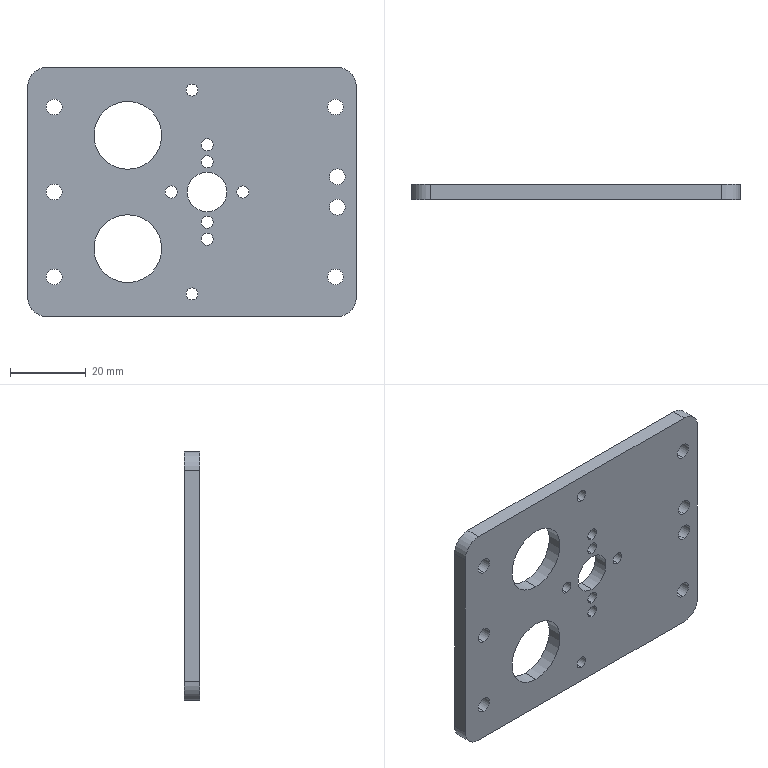Part | SolidWorks | features BaseBody 1 | 1 solid | 46 faces | box 87 x 4 x 66 mm | volume 19855 mm3 | cylinder 40 | plane 6 | commonest cylinder face diameters 3.2 x16 4.2 x14 10 x4 18 x4 10.5 x2
STEP:
#1=CARTESIAN_POINT('',(38.5,4.,6.1));
#2=VERTEX_POINT('',#1);
#3=CARTESIAN_POINT('',(38.5,4.,1.9));
#4=VERTEX_POINT('',#3);
#5=CARTESIAN_POINT('',(38.5,4.,4.));
#6=DIRECTION('',(0.,-1.,0.));
#7=DIRECTION('',(0.,0.,-1.));
#8=AXIS2_PLACEMENT_3D('',#5,#6,#7);
#9=CIRCLE('',#8,2.1);
#10=EDGE_CURVE('',#2,#4,#9,.T.);
#11=ORIENTED_EDGE('',*,*,#10,.F.);
#12=CARTESIAN_POINT('',(38.5,0.,6.1));
#13=VERTEX_POINT('',#12);
#14=CARTESIAN_POINT('',(38.5,4.,6.1));
#15=DIRECTION('',(0.,-1.,0.));
#16=VECTOR('',#15,1000.);
#17=LINE('',#14,#16);
#18=EDGE_CURVE('',#2,#13,#17,.T.);
#19=ORIENTED_EDGE('',*,*,#18,.T.);
#20=CARTESIAN_POINT('',(38.5,0.,1.9));
#21=VERTEX_POINT('',#20);
#22=CARTESIAN_POINT('',(38.5,0.,4.));
#23=DIRECTION('',(0.,-1.,0.));
#24=DIRECTION('',(0.,0.,-1.));
#25=AXIS2_PLACEMENT_3D('',#22,#23,#24);
#26=CIRCLE('',#25,2.1);
#27=EDGE_CURVE('',#13,#21,#26,.T.);
#28=ORIENTED_EDGE('',*,*,#27,.T.);
#29=CARTESIAN_POINT('',(38.5,4.,1.9));
#30=DIRECTION('',(0.,-1.,0.));
#31=VECTOR('',#30,1000.);
#32=LINE('',#29,#31);
#33=EDGE_CURVE('',#4,#21,#32,.T.);
#34=ORIENTED_EDGE('',*,*,#33,.F.);
#35=EDGE_LOOP('',(#11,#19,#28,#34));
#36=FACE_OUTER_BOUND('',#35,.T.);
#37=CARTESIAN_POINT('',(38.5,4.,4.));
#38=DIRECTION('',(0.,-1.,0.));
#39=DIRECTION('',(0.,0.,-1.));
#40=AXIS2_PLACEMENT_3D('',#37,#38,#39);
#41=CYLINDRICAL_SURFACE('',#40,2.1);
#42=ADVANCED_FACE('',(#36),#41,.F.);
#43=CARTESIAN_POINT('',(38.5,4.,-1.9));
#44=VERTEX_POINT('',#43);
#45=CARTESIAN_POINT('',(38.5,4.,-6.1));
#46=VERTEX_POINT('',#45);
#47=CARTESIAN_POINT('',(38.5,4.,-4.));
#48=DIRECTION('',(0.,-1.,0.));
#49=DIRECTION('',(0.,0.,-1.));
#50=AXIS2_PLACEMENT_3D('',#47,#48,#49);
#51=CIRCLE('',#50,2.1);
#52=EDGE_CURVE('',#44,#46,#51,.T.);
#53=ORIENTED_EDGE('',*,*,#52,.F.);
#54=CARTESIAN_POINT('',(38.5,0.,-1.9));
#55=VERTEX_POINT('',#54);
#56=CARTESIAN_POINT('',(38.5,4.,-1.9));
#57=DIRECTION('',(0.,-1.,0.));
#58=VECTOR('',#57,1000.);
#59=LINE('',#56,#58);
#60=EDGE_CURVE('',#44,#55,#59,.T.);
#61=ORIENTED_EDGE('',*,*,#60,.T.);
#62=CARTESIAN_POINT('',(38.5,0.,-6.1));
#63=VERTEX_POINT('',#62);
#64=CARTESIAN_POINT('',(38.5,0.,-4.));
#65=DIRECTION('',(0.,-1.,0.));
#66=DIRECTION('',(0.,0.,-1.));
#67=AXIS2_PLACEMENT_3D('',#64,#65,#66);
#68=CIRCLE('',#67,2.1);
#69=EDGE_CURVE('',#55,#63,#68,.T.);
#70=ORIENTED_EDGE('',*,*,#69,.T.);
#71=CARTESIAN_POINT('',(38.5,4.,-6.1));
#72=DIRECTION('',(0.,-1.,0.));
#73=VECTOR('',#72,1000.);
#74=LINE('',#71,#73);
#75=EDGE_CURVE('',#46,#63,#74,.T.);
#76=ORIENTED_EDGE('',*,*,#75,.F.);
#77=EDGE_LOOP('',(#53,#61,#70,#76));
#78=FACE_OUTER_BOUND('',#77,.T.);
#79=CARTESIAN_POINT('',(38.5,4.,-4.));
#80=DIRECTION('',(0.,-1.,0.));
#81=DIRECTION('',(0.,0.,-1.));
#82=AXIS2_PLACEMENT_3D('',#79,#80,#81);
#83=CYLINDRICAL_SURFACE('',#82,2.1);
#84=ADVANCED_FACE('',(#78),#83,.F.);
#85=CARTESIAN_POINT('',(0.,4.,28.6));
#86=VERTEX_POINT('',#85);
#87=CARTESIAN_POINT('',(0.,4.,25.4));
#88=VERTEX_POINT('',#87);
#89=CARTESIAN_POINT('',(0.,4.,27.));
#90=DIRECTION('',(0.,-1.,0.));
#91=DIRECTION('',(0.,0.,-1.));
#92=AXIS2_PLACEMENT_3D('',#89,#90,#91);
#93=CIRCLE('',#92,1.6);
#94=EDGE_CURVE('',#86,#88,#93,.T.);
#95=ORIENTED_EDGE('',*,*,#94,.F.);
#96=CARTESIAN_POINT('',(0.,0.,28.6));
#97=VERTEX_POINT('',#96);
#98=CARTESIAN_POINT('',(0.,4.,28.6));
#99=DIRECTION('',(0.,-1.,0.));
#100=VECTOR('',#99,1000.);
#101=LINE('',#98,#100);
#102=EDGE_CURVE('',#86,#97,#101,.T.);
#103=ORIENTED_EDGE('',*,*,#102,.T.);
#104=CARTESIAN_POINT('',(0.,0.,25.4));
#105=VERTEX_POINT('',#104);
#106=CARTESIAN_POINT('',(0.,0.,27.));
#107=DIRECTION('',(0.,-1.,0.));
#108=DIRECTION('',(0.,0.,-1.));
#109=AXIS2_PLACEMENT_3D('',#106,#107,#108);
#110=CIRCLE('',#109,1.6);
#111=EDGE_CURVE('',#97,#105,#110,.T.);
#112=ORIENTED_EDGE('',*,*,#111,.T.);
#113=CARTESIAN_POINT('',(0.,4.,25.4));
#114=DIRECTION('',(0.,-1.,0.));
#115=VECTOR('',#114,1000.);
#116=LINE('',#113,#115);
#117=EDGE_CURVE('',#88,#105,#116,.T.);
#118=ORIENTED_EDGE('',*,*,#117,.F.);
#119=EDGE_LOOP('',(#95,#103,#112,#118));
#120=FACE_OUTER_BOUND('',#119,.T.);
#121=CARTESIAN_POINT('',(0.,4.,27.));
#122=DIRECTION('',(0.,-1.,0.));
#123=DIRECTION('',(0.,0.,-1.));
#124=AXIS2_PLACEMENT_3D('',#121,#122,#123);
#125=CYLINDRICAL_SURFACE('',#124,1.6);
#126=ADVANCED_FACE('',(#120),#125,.F.);
#127=CARTESIAN_POINT('',(38.,4.,-20.4));
#128=VERTEX_POINT('',#127);
#129=CARTESIAN_POINT('',(38.,4.,-24.6));
#130=VERTEX_POINT('',#129);
#131=CARTESIAN_POINT('',(38.,4.,-22.5));
#132=DIRECTION('',(0.,-1.,0.));
#133=DIRECTION('',(0.,0.,-1.));
#134=AXIS2_PLACEMENT_3D('',#131,#132,#133);
#135=CIRCLE('',#134,2.1);
#136=EDGE_CURVE('',#128,#130,#135,.T.);
#137=ORIENTED_EDGE('',*,*,#136,.F.);
#138=CARTESIAN_POINT('',(38.,0.,-20.4));
#139=VERTEX_POINT('',#138);
#140=CARTESIAN_POINT('',(38.,4.,-20.4));
#141=DIRECTION('',(0.,-1.,0.));
#142=VECTOR('',#141,1000.);
#143=LINE('',#140,#142);
#144=EDGE_CURVE('',#128,#139,#143,.T.);
#145=ORIENTED_EDGE('',*,*,#144,.T.);
#146=CARTESIAN_POINT('',(38.,0.,-24.6));
#147=VERTEX_POINT('',#146);
#148=CARTESIAN_POINT('',(38.,0.,-22.5));
#149=DIRECTION('',(0.,-1.,0.));
#150=DIRECTION('',(0.,0.,-1.));
#151=AXIS2_PLACEMENT_3D('',#148,#149,#150);
#152=CIRCLE('',#151,2.1);
#153=EDGE_CURVE('',#139,#147,#152,.T.);
#154=ORIENTED_EDGE('',*,*,#153,.T.);
#155=CARTESIAN_POINT('',(38.,4.,-24.6));
#156=DIRECTION('',(0.,-1.,0.));
#157=VECTOR('',#156,1000.);
#158=LINE('',#155,#157);
#159=EDGE_CURVE('',#130,#147,#158,.T.);
#160=ORIENTED_EDGE('',*,*,#159,.F.);
#161=EDGE_LOOP('',(#137,#145,#154,#160));
#162=FACE_OUTER_BOUND('',#161,.T.);
#163=CARTESIAN_POINT('',(38.,4.,-22.5));
#164=DIRECTION('',(0.,-1.,0.));
#165=DIRECTION('',(0.,0.,-1.));
#166=AXIS2_PLACEMENT_3D('',#163,#164,#165);
#167=CYLINDRICAL_SURFACE('',#166,2.1);
#168=ADVANCED_FACE('',(#162),#167,.F.);
#169=CARTESIAN_POINT('',(38.,4.,24.6));
#170=VERTEX_POINT('',#169);
#171=CARTESIAN_POINT('',(38.,4.,20.4));
#172=VERTEX_POINT('',#171);
#173=CARTESIAN_POINT('',(38.,4.,22.5));
#174=DIRECTION('',(0.,-1.,0.));
#175=DIRECTION('',(0.,0.,-1.));
#176=AXIS2_PLACEMENT_3D('',#173,#174,#175);
#177=CIRCLE('',#176,2.1);
#178=EDGE_CURVE('',#170,#172,#177,.T.);
#179=ORIENTED_EDGE('',*,*,#178,.F.);
#180=CARTESIAN_POINT('',(38.,0.,24.6));
#181=VERTEX_POINT('',#180);
#182=CARTESIAN_POINT('',(38.,4.,24.6));
#183=DIRECTION('',(0.,-1.,0.));
#184=VECTOR('',#183,1000.);
#185=LINE('',#182,#184);
#186=EDGE_CURVE('',#170,#181,#185,.T.);
#187=ORIENTED_EDGE('',*,*,#186,.T.);
#188=CARTESIAN_POINT('',(38.,0.,20.4));
#189=VERTEX_POINT('',#188);
#190=CARTESIAN_POINT('',(38.,0.,22.5));
#191=DIRECTION('',(0.,-1.,0.));
#192=DIRECTION('',(0.,0.,-1.));
#193=AXIS2_PLACEMENT_3D('',#190,#191,#192);
#194=CIRCLE('',#193,2.1);
#195=EDGE_CURVE('',#181,#189,#194,.T.);
#196=ORIENTED_EDGE('',*,*,#195,.T.);
#197=CARTESIAN_POINT('',(38.,4.,20.4));
#198=DIRECTION('',(0.,-1.,0.));
#199=VECTOR('',#198,1000.);
#200=LINE('',#197,#199);
#201=EDGE_CURVE('',#172,#189,#200,.T.);
#202=ORIENTED_EDGE('',*,*,#201,.F.);
#203=EDGE_LOOP('',(#179,#187,#196,#202));
#204=FACE_OUTER_BOUND('',#203,.T.);
#205=CARTESIAN_POINT('',(38.,4.,22.5));
#206=DIRECTION('',(0.,-1.,0.));
#207=DIRECTION('',(0.,0.,-1.));
#208=AXIS2_PLACEMENT_3D('',#205,#206,#207);
#209=CYLINDRICAL_SURFACE('',#208,2.1);
#210=ADVANCED_FACE('',(#204),#209,.F.);
#211=CARTESIAN_POINT('',(-36.5,4.,24.6));
#212=VERTEX_POINT('',#211);
#213=CARTESIAN_POINT('',(-36.5,4.,20.4));
#214=VERTEX_POINT('',#213);
#215=CARTESIAN_POINT('',(-36.5,4.,22.5));
#216=DIRECTION('',(0.,-1.,0.));
#217=DIRECTION('',(0.,0.,-1.));
#218=AXIS2_PLACEMENT_3D('',#215,#216,#217);
#219=CIRCLE('',#218,2.1);
#220=EDGE_CURVE('',#212,#214,#219,.T.);
#221=ORIENTED_EDGE('',*,*,#220,.F.);
#222=CARTESIAN_POINT('',(-36.5,0.,24.6));
#223=VERTEX_POINT('',#222);
#224=CARTESIAN_POINT('',(-36.5,4.,24.6));
#225=DIRECTION('',(0.,-1.,0.));
#226=VECTOR('',#225,1000.);
#227=LINE('',#224,#226);
#228=EDGE_CURVE('',#212,#223,#227,.T.);
#229=ORIENTED_EDGE('',*,*,#228,.T.);
#230=CARTESIAN_POINT('',(-36.5,0.,20.4));
#231=VERTEX_POINT('',#230);
#232=CARTESIAN_POINT('',(-36.5,0.,22.5));
#233=DIRECTION('',(0.,-1.,0.));
#234=DIRECTION('',(0.,0.,-1.));
#235=AXIS2_PLACEMENT_3D('',#232,#233,#234);
#236=CIRCLE('',#235,2.1);
#237=EDGE_CURVE('',#223,#231,#236,.T.);
#238=ORIENTED_EDGE('',*,*,#237,.T.);
#239=CARTESIAN_POINT('',(-36.5,4.,20.4));
#240=DIRECTION('',(0.,-1.,0.));
#241=VECTOR('',#240,1000.);
#242=LINE('',#239,#241);
#243=EDGE_CURVE('',#214,#231,#242,.T.);
#244=ORIENTED_EDGE('',*,*,#243,.F.);
#245=EDGE_LOOP('',(#221,#229,#238,#244));
#246=FACE_OUTER_BOUND('',#245,.T.);
#247=CARTESIAN_POINT('',(-36.5,4.,22.5));
#248=DIRECTION('',(0.,-1.,0.));
#249=DIRECTION('',(0.,0.,-1.));
#250=AXIS2_PLACEMENT_3D('',#247,#248,#249);
#251=CYLINDRICAL_SURFACE('',#250,2.1);
#252=ADVANCED_FACE('',(#246),#251,.F.);
#253=CARTESIAN_POINT('',(-36.5,4.,2.1));
#254=VERTEX_POINT('',#253);
#255=CARTESIAN_POINT('',(-36.5,4.,-2.1));
#256=VERTEX_POINT('',#255);
#257=CARTESIAN_POINT('',(-36.5,4.,0.));
#258=DIRECTION('',(0.,-1.,0.));
#259=DIRECTION('',(0.,0.,-1.));
#260=AXIS2_PLACEMENT_3D('',#257,#258,#259);
#261=CIRCLE('',#260,2.1);
#262=EDGE_CURVE('',#254,#256,#261,.T.);
#263=ORIENTED_EDGE('',*,*,#262,.F.);
#264=CARTESIAN_POINT('',(-36.5,0.,2.1));
#265=VERTEX_POINT('',#264);
#266=CARTESIAN_POINT('',(-36.5,4.,2.1));
#267=DIRECTION('',(0.,-1.,0.));
#268=VECTOR('',#267,1000.);
#269=LINE('',#266,#268);
#270=EDGE_CURVE('',#254,#265,#269,.T.);
#271=ORIENTED_EDGE('',*,*,#270,.T.);
#272=CARTESIAN_POINT('',(-36.5,0.,-2.1));
#273=VERTEX_POINT('',#272);
#274=CARTESIAN_POINT('',(-36.5,0.,0.));
#275=DIRECTION('',(0.,-1.,0.));
#276=DIRECTION('',(0.,0.,-1.));
#277=AXIS2_PLACEMENT_3D('',#274,#275,#276);
#278=CIRCLE('',#277,2.1);
#279=EDGE_CURVE('',#265,#273,#278,.T.);
#280=ORIENTED_EDGE('',*,*,#279,.T.);
#281=CARTESIAN_POINT('',(-36.5,4.,-2.1));
#282=DIRECTION('',(0.,-1.,0.));
#283=VECTOR('',#282,1000.);
#284=LINE('',#281,#283);
#285=EDGE_CURVE('',#256,#273,#284,.T.);
#286=ORIENTED_EDGE('',*,*,#285,.F.);
#287=EDGE_LOOP('',(#263,#271,#280,#286));
#288=FACE_OUTER_BOUND('',#287,.T.);
#289=CARTESIAN_POINT('',(-36.5,4.,0.));
#290=DIRECTION('',(0.,-1.,0.));
#291=DIRECTION('',(0.,0.,-1.));
#292=AXIS2_PLACEMENT_3D('',#289,#290,#291);
#293=CYLINDRICAL_SURFACE('',#292,2.1);
#294=ADVANCED_FACE('',(#288),#293,.F.);
#295=CARTESIAN_POINT('',(-36.5,4.,-20.4));
#296=VERTEX_POINT('',#295);
#297=CARTESIAN_POINT('',(-36.5,4.,-24.6));
#298=VERTEX_POINT('',#297);
#299=CARTESIAN_POINT('',(-36.5,4.,-22.5));
#300=DIRECTION('',(0.,-1.,0.));
#301=DIRECTION('',(0.,0.,-1.));
#302=AXIS2_PLACEMENT_3D('',#299,#300,#301);
#303=CIRCLE('',#302,2.1);
#304=EDGE_CURVE('',#296,#298,#303,.T.);
#305=ORIENTED_EDGE('',*,*,#304,.F.);
#306=CARTESIAN_POINT('',(-36.5,0.,-20.4));
#307=VERTEX_POINT('',#306);
#308=CARTESIAN_POINT('',(-36.5,4.,-20.4));
#309=DIRECTION('',(0.,-1.,0.));
#310=VECTOR('',#309,1000.);
#311=LINE('',#308,#310);
#312=EDGE_CURVE('',#296,#307,#311,.T.);
#313=ORIENTED_EDGE('',*,*,#312,.T.);
#314=CARTESIAN_POINT('',(-36.5,0.,-24.6));
#315=VERTEX_POINT('',#314);
#316=CARTESIAN_POINT('',(-36.5,0.,-22.5));
#317=DIRECTION('',(0.,-1.,0.));
#318=DIRECTION('',(0.,0.,-1.));
#319=AXIS2_PLACEMENT_3D('',#316,#317,#318);
#320=CIRCLE('',#319,2.1);
#321=EDGE_CURVE('',#307,#315,#320,.T.);
#322=ORIENTED_EDGE('',*,*,#321,.T.);
#323=CARTESIAN_POINT('',(-36.5,4.,-24.6));
#324=DIRECTION('',(0.,-1.,0.));
#325=VECTOR('',#324,1000.);
#326=LINE('',#323,#325);
#327=EDGE_CURVE('',#298,#315,#326,.T.);
#328=ORIENTED_EDGE('',*,*,#327,.F.);
#329=EDGE_LOOP('',(#305,#313,#322,#328));
#330=FACE_OUTER_BOUND('',#329,.T.);
#331=CARTESIAN_POINT('',(-36.5,4.,-22.5));
#332=DIRECTION('',(0.,-1.,0.));
#333=DIRECTION('',(0.,0.,-1.));
#334=AXIS2_PLACEMENT_3D('',#331,#332,#333);
#335=CYLINDRICAL_SURFACE('',#334,2.1);
#336=ADVANCED_FACE('',(#330),#335,.F.);
#337=CARTESIAN_POINT('',(0.,4.,-25.4));
#338=VERTEX_POINT('',#337);
#339=CARTESIAN_POINT('',(0.,4.,-28.6));
#340=VERTEX_POINT('',#339);
#341=CARTESIAN_POINT('',(0.,4.,-27.));
#342=DIRECTION('',(0.,-1.,0.));
#343=DIRECTION('',(0.,0.,-1.));
#344=AXIS2_PLACEMENT_3D('',#341,#342,#343);
#345=CIRCLE('',#344,1.6);
#346=EDGE_CURVE('',#338,#340,#345,.T.);
#347=ORIENTED_EDGE('',*,*,#346,.F.);
#348=CARTESIAN_POINT('',(0.,0.,-25.4));
#349=VERTEX_POINT('',#348);
#350=CARTESIAN_POINT('',(0.,4.,-25.4));
#351=DIRECTION('',(0.,-1.,0.));
#352=VECTOR('',#351,1000.);
#353=LINE('',#350,#352);
#354=EDGE_CURVE('',#338,#349,#353,.T.);
#355=ORIENTED_EDGE('',*,*,#354,.T.);
#356=CARTESIAN_POINT('',(0.,0.,-28.6));
#357=VERTEX_POINT('',#356);
#358=CARTESIAN_POINT('',(0.,0.,-27.));
#359=DIRECTION('',(0.,-1.,0.));
#360=DIRECTION('',(0.,0.,-1.));
#361=AXIS2_PLACEMENT_3D('',#358,#359,#360);
#362=CIRCLE('',#361,1.6);
#363=EDGE_CURVE('',#349,#357,#362,.T.);
#364=ORIENTED_EDGE('',*,*,#363,.T.);
#365=CARTESIAN_POINT('',(0.,4.,-28.6));
#366=DIRECTION('',(0.,-1.,0.));
#367=VECTOR('',#366,1000.);
#368=LINE('',#365,#367);
#369=EDGE_CURVE('',#340,#357,#368,.T.);
#370=ORIENTED_EDGE('',*,*,#369,.F.);
#371=EDGE_LOOP('',(#347,#355,#364,#370));
#372=FACE_OUTER_BOUND('',#371,.T.);
#373=CARTESIAN_POINT('',(0.,4.,-27.));
#374=DIRECTION('',(0.,-1.,0.));
#375=DIRECTION('',(0.,0.,-1.));
#376=AXIS2_PLACEMENT_3D('',#373,#374,#375);
#377=CYLINDRICAL_SURFACE('',#376,1.6);
#378=ADVANCED_FACE('',(#372),#377,.F.);
#379=CARTESIAN_POINT('',(4.,4.,5.25));
#380=VERTEX_POINT('',#379);
#381=CARTESIAN_POINT('',(4.,4.,-5.25));
#382=VERTEX_POINT('',#381);
#383=CARTESIAN_POINT('',(4.,4.,0.));
#384=DIRECTION('',(0.,-1.,0.));
#385=DIRECTION('',(0.,0.,-1.));
#386=AXIS2_PLACEMENT_3D('',#383,#384,#385);
#387=CIRCLE('',#386,5.25);
#388=EDGE_CURVE('',#380,#382,#387,.T.);
#389=ORIENTED_EDGE('',*,*,#388,.F.);
#390=CARTESIAN_POINT('',(4.,0.,5.25));
#391=VERTEX_POINT('',#390);
#392=CARTESIAN_POINT('',(4.,4.,5.25));
#393=DIRECTION('',(0.,-1.,0.));
#394=VECTOR('',#393,1000.);
#395=LINE('',#392,#394);
#396=EDGE_CURVE('',#380,#391,#395,.T.);
#397=ORIENTED_EDGE('',*,*,#396,.T.);
#398=CARTESIAN_POINT('',(4.,0.,-5.25));
#399=VERTEX_POINT('',#398);
#400=CARTESIAN_POINT('',(4.,0.,0.));
#401=DIRECTION('',(0.,-1.,0.));
#402=DIRECTION('',(0.,0.,-1.));
#403=AXIS2_PLACEMENT_3D('',#400,#401,#402);
#404=CIRCLE('',#403,5.25);
#405=EDGE_CURVE('',#391,#399,#404,.T.);
#406=ORIENTED_EDGE('',*,*,#405,.T.);
#407=CARTESIAN_POINT('',(4.,4.,-5.25));
#408=DIRECTION('',(0.,-1.,0.));
#409=VECTOR('',#408,1000.);
#410=LINE('',#407,#409);
#411=EDGE_CURVE('',#382,#399,#410,.T.);
#412=ORIENTED_EDGE('',*,*,#411,.F.);
#413=EDGE_LOOP('',(#389,#397,#406,#412));
#414=FACE_OUTER_BOUND('',#413,.T.);
#415=CARTESIAN_POINT('',(4.,4.,0.));
#416=DIRECTION('',(0.,-1.,0.));
#417=DIRECTION('',(0.,0.,-1.));
#418=AXIS2_PLACEMENT_3D('',#415,#416,#417);
#419=CYLINDRICAL_SURFACE('',#418,5.25);
#420=ADVANCED_FACE('',(#414),#419,.F.);
#421=CARTESIAN_POINT('',(4.,4.,14.1));
#422=VERTEX_POINT('',#421);
#423=CARTESIAN_POINT('',(4.,4.,10.9));
#424=VERTEX_POINT('',#423);
#425=CARTESIAN_POINT('',(4.,4.,12.5));
#426=DIRECTION('',(0.,-1.,0.));
#427=DIRECTION('',(0.,0.,-1.));
#428=AXIS2_PLACEMENT_3D('',#425,#426,#427);
#429=CIRCLE('',#428,1.6);
#430=EDGE_CURVE('',#422,#424,#429,.T.);
#431=ORIENTED_EDGE('',*,*,#430,.F.);
#432=CARTESIAN_POINT('',(4.,0.,14.1));
#433=VERTEX_POINT('',#432);
#434=CARTESIAN_POINT('',(4.,4.,14.1));
#435=DIRECTION('',(0.,-1.,0.));
#436=VECTOR('',#435,1000.);
#437=LINE('',#434,#436);
#438=EDGE_CURVE('',#422,#433,#437,.T.);
#439=ORIENTED_EDGE('',*,*,#438,.T.);
#440=CARTESIAN_POINT('',(4.,0.,10.9));
#441=VERTEX_POINT('',#440);
#442=CARTESIAN_POINT('',(4.,0.,12.5));
#443=DIRECTION('',(0.,-1.,0.));
#444=DIRECTION('',(0.,0.,-1.));
#445=AXIS2_PLACEMENT_3D('',#442,#443,#444);
#446=CIRCLE('',#445,1.6);
#447=EDGE_CURVE('',#433,#441,#446,.T.);
#448=ORIENTED_EDGE('',*,*,#447,.T.);
#449=CARTESIAN_POINT('',(4.,4.,10.9));
#450=DIRECTION('',(0.,-1.,0.));
#451=VECTOR('',#450,1000.);
#452=LINE('',#449,#451);
#453=EDGE_CURVE('',#424,#441,#452,.T.);
#454=ORIENTED_EDGE('',*,*,#453,.F.);
#455=EDGE_LOOP('',(#431,#439,#448,#454));
#456=FACE_OUTER_BOUND('',#455,.T.);
#457=CARTESIAN_POINT('',(4.,4.,12.5));
#458=DIRECTION('',(0.,-1.,0.));
#459=DIRECTION('',(0.,0.,-1.));
#460=AXIS2_PLACEMENT_3D('',#457,#458,#459);
#461=CYLINDRICAL_SURFACE('',#460,1.6);
#462=ADVANCED_FACE('',(#456),#461,.F.);
#463=CARTESIAN_POINT('',(4.,4.,-10.9));
#464=VERTEX_POINT('',#463);
#465=CARTESIAN_POINT('',(4.,4.,-14.1));
#466=VERTEX_POINT('',#465);
#467=CARTESIAN_POINT('',(4.,4.,-12.5));
#468=DIRECTION('',(0.,-1.,0.));
#469=DIRECTION('',(0.,0.,-1.));
#470=AXIS2_PLACEMENT_3D('',#467,#468,#469);
#471=CIRCLE('',#470,1.6);
#472=EDGE_CURVE('',#464,#466,#471,.T.);
#473=ORIENTED_EDGE('',*,*,#472,.F.);
#474=CARTESIAN_POINT('',(4.,0.,-10.9));
#475=VERTEX_POINT('',#474);
#476=CARTESIAN_POINT('',(4.,4.,-10.9));
#477=DIRECTION('',(0.,-1.,0.));
#478=VECTOR('',#477,1000.);
#479=LINE('',#476,#478);
#480=EDGE_CURVE('',#464,#475,#479,.T.);
#481=ORIENTED_EDGE('',*,*,#480,.T.);
#482=CARTESIAN_POINT('',(4.,0.,-14.1));
#483=VERTEX_POINT('',#482);
#484=CARTESIAN_POINT('',(4.,0.,-12.5));
#485=DIRECTION('',(0.,-1.,0.));
#486=DIRECTION('',(0.,0.,-1.));
#487=AXIS2_PLACEMENT_3D('',#484,#485,#486);
#488=CIRCLE('',#487,1.6);
#489=EDGE_CURVE('',#475,#483,#488,.T.);
#490=ORIENTED_EDGE('',*,*,#489,.T.);
#491=CARTESIAN_POINT('',(4.,4.,-14.1));
#492=DIRECTION('',(0.,-1.,0.));
#493=VECTOR('',#492,1000.);
#494=LINE('',#491,#493);
#495=EDGE_CURVE('',#466,#483,#494,.T.);
#496=ORIENTED_EDGE('',*,*,#495,.F.);
#497=EDGE_LOOP('',(#473,#481,#490,#496));
#498=FACE_OUTER_BOUND('',#497,.T.);
#499=CARTESIAN_POINT('',(4.,4.,-12.5));
#500=DIRECTION('',(0.,-1.,0.));
#501=DIRECTION('',(0.,0.,-1.));
#502=AXIS2_PLACEMENT_3D('',#499,#500,#501);
#503=CYLINDRICAL_SURFACE('',#502,1.6);
#504=ADVANCED_FACE('',(#498),#503,.F.);
#505=CARTESIAN_POINT('',(4.,4.,-6.4));
#506=VERTEX_POINT('',#505);
#507=CARTESIAN_POINT('',(4.,4.,-9.6));
#508=VERTEX_POINT('',#507);
#509=CARTESIAN_POINT('',(4.,4.,-8.));
#510=DIRECTION('',(0.,-1.,0.));
#511=DIRECTION('',(0.,0.,-1.));
#512=AXIS2_PLACEMENT_3D('',#509,#510,#511);
#513=CIRCLE('',#512,1.6);
#514=EDGE_CURVE('',#506,#508,#513,.T.);
#515=ORIENTED_EDGE('',*,*,#514,.F.);
#516=CARTESIAN_POINT('',(4.,0.,-6.4));
#517=VERTEX_POINT('',#516);
#518=CARTESIAN_POINT('',(4.,4.,-6.4));
#519=DIRECTION('',(0.,-1.,0.));
#520=VECTOR('',#519,1000.);
#521=LINE('',#518,#520);
#522=EDGE_CURVE('',#506,#517,#521,.T.);
#523=ORIENTED_EDGE('',*,*,#522,.T.);
#524=CARTESIAN_POINT('',(4.,0.,-9.6));
#525=VERTEX_POINT('',#524);
#526=CARTESIAN_POINT('',(4.,0.,-8.));
#527=DIRECTION('',(0.,-1.,0.));
#528=DIRECTION('',(0.,0.,-1.));
#529=AXIS2_PLACEMENT_3D('',#526,#527,#528);
#530=CIRCLE('',#529,1.6);
#531=EDGE_CURVE('',#517,#525,#530,.T.);
#532=ORIENTED_EDGE('',*,*,#531,.T.);
#533=CARTESIAN_POINT('',(4.,4.,-9.6));
#534=DIRECTION('',(0.,-1.,0.));
#535=VECTOR('',#534,1000.);
#536=LINE('',#533,#535);
#537=EDGE_CURVE('',#508,#525,#536,.T.);
#538=ORIENTED_EDGE('',*,*,#537,.F.);
#539=EDGE_LOOP('',(#515,#523,#532,#538));
#540=FACE_OUTER_BOUND('',#539,.T.);
#541=CARTESIAN_POINT('',(4.,4.,-8.));
#542=DIRECTION('',(0.,-1.,0.));
#543=DIRECTION('',(0.,0.,-1.));
#544=AXIS2_PLACEMENT_3D('',#541,#542,#543);
#545=CYLINDRICAL_SURFACE('',#544,1.6);
#546=ADVANCED_FACE('',(#540),#545,.F.);
#547=CARTESIAN_POINT('',(4.,4.,9.6));
#548=VERTEX_POINT('',#547);
#549=CARTESIAN_POINT('',(4.,4.,6.4));
#550=VERTEX_POINT('',#549);
#551=CARTESIAN_POINT('',(4.,4.,8.));
#552=DIRECTION('',(0.,-1.,0.));
#553=DIRECTION('',(0.,0.,-1.));
#554=AXIS2_PLACEMENT_3D('',#551,#552,#553);
#555=CIRCLE('',#554,1.6);
#556=EDGE_CURVE('',#548,#550,#555,.T.);
#557=ORIENTED_EDGE('',*,*,#556,.F.);
#558=CARTESIAN_POINT('',(4.,0.,9.6));
#559=VERTEX_POINT('',#558);
#560=CARTESIAN_POINT('',(4.,4.,9.6));
#561=DIRECTION('',(0.,-1.,0.));
#562=VECTOR('',#561,1000.);
#563=LINE('',#560,#562);
#564=EDGE_CURVE('',#548,#559,#563,.T.);
#565=ORIENTED_EDGE('',*,*,#564,.T.);
#566=CARTESIAN_POINT('',(4.,0.,6.4));
#567=VERTEX_POINT('',#566);
#568=CARTESIAN_POINT('',(4.,0.,8.));
#569=DIRECTION('',(0.,-1.,0.));
#570=DIRECTION('',(0.,0.,-1.));
#571=AXIS2_PLACEMENT_3D('',#568,#569,#570);
#572=CIRCLE('',#571,1.6);
#573=EDGE_CURVE('',#559,#567,#572,.T.);
#574=ORIENTED_EDGE('',*,*,#573,.T.);
#575=CARTESIAN_POINT('',(4.,4.,6.4));
#576=DIRECTION('',(0.,-1.,0.));
#577=VECTOR('',#576,1000.);
#578=LINE('',#575,#577);
#579=EDGE_CURVE('',#550,#567,#578,.T.);
#580=ORIENTED_EDGE('',*,*,#579,.F.);
#581=EDGE_LOOP('',(#557,#565,#574,#580));
#582=FACE_OUTER_BOUND('',#581,.T.);
#583=CARTESIAN_POINT('',(4.,4.,8.));
#584=DIRECTION('',(0.,-1.,0.));
#585=DIRECTION('',(0.,0.,-1.));
#586=AXIS2_PLACEMENT_3D('',#583,#584,#585);
#587=CYLINDRICAL_SURFACE('',#586,1.6);
#588=ADVANCED_FACE('',(#582),#587,.F.);
#589=CARTESIAN_POINT('',(13.5,4.,1.6));
#590=VERTEX_POINT('',#589);
#591=CARTESIAN_POINT('',(13.5,4.,-1.6));
#592=VERTEX_POINT('',#591);
#593=CARTESIAN_POINT('',(13.5,4.,0.));
#594=DIRECTION('',(0.,-1.,0.));
#595=DIRECTION('',(0.,0.,-1.));
#596=AXIS2_PLACEMENT_3D('',#593,#594,#595);
#597=CIRCLE('',#596,1.6);
#598=EDGE_CURVE('',#590,#592,#597,.T.);
#599=ORIENTED_EDGE('',*,*,#598,.F.);
#600=CARTESIAN_POINT('',(13.5,0.,1.6));
#601=VERTEX_POINT('',#600);
#602=CARTESIAN_POINT('',(13.5,4.,1.6));
#603=DIRECTION('',(0.,-1.,0.));
#604=VECTOR('',#603,1000.);
#605=LINE('',#602,#604);
#606=EDGE_CURVE('',#590,#601,#605,.T.);
#607=ORIENTED_EDGE('',*,*,#606,.T.);
#608=CARTESIAN_POINT('',(13.5,0.,-1.6));
#609=VERTEX_POINT('',#608);
#610=CARTESIAN_POINT('',(13.5,0.,0.));
#611=DIRECTION('',(0.,-1.,0.));
#612=DIRECTION('',(0.,0.,-1.));
#613=AXIS2_PLACEMENT_3D('',#610,#611,#612);
#614=CIRCLE('',#613,1.6);
#615=EDGE_CURVE('',#601,#609,#614,.T.);
#616=ORIENTED_EDGE('',*,*,#615,.T.);
#617=CARTESIAN_POINT('',(13.5,4.,-1.6));
#618=DIRECTION('',(0.,-1.,0.));
#619=VECTOR('',#618,1000.);
#620=LINE('',#617,#619);
#621=EDGE_CURVE('',#592,#609,#620,.T.);
#622=ORIENTED_EDGE('',*,*,#621,.F.);
#623=EDGE_LOOP('',(#599,#607,#616,#622));
#624=FACE_OUTER_BOUND('',#623,.T.);
#625=CARTESIAN_POINT('',(13.5,4.,0.));
#626=DIRECTION('',(0.,-1.,0.));
#627=DIRECTION('',(0.,0.,-1.));
#628=AXIS2_PLACEMENT_3D('',#625,#626,#627);
#629=CYLINDRICAL_SURFACE('',#628,1.6);
#630=ADVANCED_FACE('',(#624),#629,.F.);
#631=CARTESIAN_POINT('',(-5.5,4.,1.6));
#632=VERTEX_POINT('',#631);
#633=CARTESIAN_POINT('',(-5.5,4.,-1.6));
#634=VERTEX_POINT('',#633);
#635=CARTESIAN_POINT('',(-5.5,4.,0.));
#636=DIRECTION('',(0.,-1.,0.));
#637=DIRECTION('',(0.,0.,-1.));
#638=AXIS2_PLACEMENT_3D('',#635,#636,#637);
#639=CIRCLE('',#638,1.6);
#640=EDGE_CURVE('',#632,#634,#639,.T.);
#641=ORIENTED_EDGE('',*,*,#640,.F.);
#642=CARTESIAN_POINT('',(-5.5,0.,1.6));
#643=VERTEX_POINT('',#642);
#644=CARTESIAN_POINT('',(-5.5,4.,1.6));
#645=DIRECTION('',(0.,-1.,0.));
#646=VECTOR('',#645,1000.);
#647=LINE('',#644,#646);
#648=EDGE_CURVE('',#632,#643,#647,.T.);
#649=ORIENTED_EDGE('',*,*,#648,.T.);
#650=CARTESIAN_POINT('',(-5.5,0.,-1.6));
#651=VERTEX_POINT('',#650);
#652=CARTESIAN_POINT('',(-5.5,0.,0.));
#653=DIRECTION('',(0.,-1.,0.));
#654=DIRECTION('',(0.,0.,-1.));
#655=AXIS2_PLACEMENT_3D('',#652,#653,#654);
#656=CIRCLE('',#655,1.6);
#657=EDGE_CURVE('',#643,#651,#656,.T.);
#658=ORIENTED_EDGE('',*,*,#657,.T.);
#659=CARTESIAN_POINT('',(-5.5,4.,-1.6));
#660=DIRECTION('',(0.,-1.,0.));
#661=VECTOR('',#660,1000.);
#662=LINE('',#659,#661);
#663=EDGE_CURVE('',#634,#651,#662,.T.);
#664=ORIENTED_EDGE('',*,*,#663,.F.);
#665=EDGE_LOOP('',(#641,#649,#658,#664));
#666=FACE_OUTER_BOUND('',#665,.T.);
#667=CARTESIAN_POINT('',(-5.5,4.,0.));
#668=DIRECTION('',(0.,-1.,0.));
#669=DIRECTION('',(0.,0.,-1.));
#670=AXIS2_PLACEMENT_3D('',#667,#668,#669);
#671=CYLINDRICAL_SURFACE('',#670,1.6);
#672=ADVANCED_FACE('',(#666),#671,.F.);
#673=CARTESIAN_POINT('',(-17.,0.,-6.));
#674=VERTEX_POINT('',#673);
#675=CARTESIAN_POINT('',(-17.,0.,-24.));
#676=VERTEX_POINT('',#675);
#677=CARTESIAN_POINT('',(-17.,0.,-15.));
#678=DIRECTION('',(0.,-1.,0.));
#679=DIRECTION('',(0.,0.,1.));
#680=AXIS2_PLACEMENT_3D('',#677,#678,#679);
#681=CIRCLE('',#680,9.);
#682=EDGE_CURVE('',#674,#676,#681,.T.);
#683=ORIENTED_EDGE('',*,*,#682,.T.);
#684=CARTESIAN_POINT('',(-17.,4.,-24.));
#685=VERTEX_POINT('',#684);
#686=CARTESIAN_POINT('',(-17.,-6.,-24.));
#687=DIRECTION('',(0.,1.,0.));
#688=VECTOR('',#687,1000.);
#689=LINE('',#686,#688);
#690=EDGE_CURVE('',#676,#685,#689,.T.);
#691=ORIENTED_EDGE('',*,*,#690,.T.);
#692=CARTESIAN_POINT('',(-17.,4.,-6.));
#693=VERTEX_POINT('',#692);
#694=CARTESIAN_POINT('',(-17.,4.,-15.));
#695=DIRECTION('',(0.,-1.,0.));
#696=DIRECTION('',(0.,0.,1.));
#697=AXIS2_PLACEMENT_3D('',#694,#695,#696);
#698=CIRCLE('',#697,9.);
#699=EDGE_CURVE('',#693,#685,#698,.T.);
#700=ORIENTED_EDGE('',*,*,#699,.F.);
#701=CARTESIAN_POINT('',(-17.,-6.,-6.));
#702=DIRECTION('',(0.,1.,0.));
#703=VECTOR('',#702,1000.);
#704=LINE('',#701,#703);
#705=EDGE_CURVE('',#674,#693,#704,.T.);
#706=ORIENTED_EDGE('',*,*,#705,.F.);
#707=EDGE_LOOP('',(#683,#691,#700,#706));
#708=FACE_OUTER_BOUND('',#707,.T.);
#709=CARTESIAN_POINT('',(-17.,-6.,-15.));
#710=DIRECTION('',(0.,1.,0.));
#711=DIRECTION('',(0.,0.,1.));
#712=AXIS2_PLACEMENT_3D('',#709,#710,#711);
#713=CYLINDRICAL_SURFACE('',#712,9.);
#714=ADVANCED_FACE('',(#708),#713,.F.);
#715=CARTESIAN_POINT('',(-17.,0.,24.));
#716=VERTEX_POINT('',#715);
#717=CARTESIAN_POINT('',(-17.,0.,6.));
#718=VERTEX_POINT('',#717);
#719=CARTESIAN_POINT('',(-17.,0.,15.));
#720=DIRECTION('',(0.,-1.,0.));
#721=DIRECTION('',(0.,0.,1.));
#722=AXIS2_PLACEMENT_3D('',#719,#720,#721);
#723=CIRCLE('',#722,9.);
#724=EDGE_CURVE('',#716,#718,#723,.T.);
#725=ORIENTED_EDGE('',*,*,#724,.T.);
#726=CARTESIAN_POINT('',(-17.,4.,6.));
#727=VERTEX_POINT('',#726);
#728=CARTESIAN_POINT('',(-17.,-6.,6.));
#729=DIRECTION('',(0.,1.,0.));
#730=VECTOR('',#729,1000.);
#731=LINE('',#728,#730);
#732=EDGE_CURVE('',#718,#727,#731,.T.);
#733=ORIENTED_EDGE('',*,*,#732,.T.);
#734=CARTESIAN_POINT('',(-17.,4.,24.));
#735=VERTEX_POINT('',#734);
#736=CARTESIAN_POINT('',(-17.,4.,15.));
#737=DIRECTION('',(0.,-1.,0.));
#738=DIRECTION('',(0.,0.,1.));
#739=AXIS2_PLACEMENT_3D('',#736,#737,#738);
#740=CIRCLE('',#739,9.);
#741=EDGE_CURVE('',#735,#727,#740,.T.);
#742=ORIENTED_EDGE('',*,*,#741,.F.);
#743=CARTESIAN_POINT('',(-17.,-6.,24.));
#744=DIRECTION('',(0.,1.,0.));
#745=VECTOR('',#744,1000.);
#746=LINE('',#743,#745);
#747=EDGE_CURVE('',#716,#735,#746,.T.);
#748=ORIENTED_EDGE('',*,*,#747,.F.);
#749=EDGE_LOOP('',(#725,#733,#742,#748));
#750=FACE_OUTER_BOUND('',#749,.T.);
#751=CARTESIAN_POINT('',(-17.,-6.,15.));
#752=DIRECTION('',(0.,1.,0.));
#753=DIRECTION('',(0.,0.,1.));
#754=AXIS2_PLACEMENT_3D('',#751,#752,#753);
#755=CYLINDRICAL_SURFACE('',#754,9.);
#756=ADVANCED_FACE('',(#750),#755,.F.);
#757=CARTESIAN_POINT('',(38.5,0.,4.));
#758=DIRECTION('',(0.,-1.,0.));
#759=DIRECTION('',(0.,0.,-1.));
#760=AXIS2_PLACEMENT_3D('',#757,#758,#759);
#761=CIRCLE('',#760,2.1);
#762=EDGE_CURVE('',#21,#13,#761,.T.);
#763=ORIENTED_EDGE('',*,*,#762,.F.);
#764=ORIENTED_EDGE('',*,*,#27,.F.);
#765=EDGE_LOOP('',(#763,#764));
#766=FACE_BOUND('',#765,.T.);
#767=CARTESIAN_POINT('',(38.5,0.,-4.));
#768=DIRECTION('',(0.,-1.,0.));
#769=DIRECTION('',(0.,0.,-1.));
#770=AXIS2_PLACEMENT_3D('',#767,#768,#769);
#771=CIRCLE('',#770,2.1);
#772=EDGE_CURVE('',#63,#55,#771,.T.);
#773=ORIENTED_EDGE('',*,*,#772,.F.);
#774=ORIENTED_EDGE('',*,*,#69,.F.);
#775=EDGE_LOOP('',(#773,#774));
#776=FACE_BOUND('',#775,.T.);
#777=CARTESIAN_POINT('',(0.,0.,27.));
#778=DIRECTION('',(0.,-1.,0.));
#779=DIRECTION('',(0.,0.,-1.));
#780=AXIS2_PLACEMENT_3D('',#777,#778,#779);
#781=CIRCLE('',#780,1.6);
#782=EDGE_CURVE('',#105,#97,#781,.T.);
#783=ORIENTED_EDGE('',*,*,#782,.F.);
#784=ORIENTED_EDGE('',*,*,#111,.F.);
#785=EDGE_LOOP('',(#783,#784));
#786=FACE_BOUND('',#785,.T.);
#787=CARTESIAN_POINT('',(38.,0.,-22.5));
#788=DIRECTION('',(0.,-1.,0.));
#789=DIRECTION('',(0.,0.,-1.));
#790=AXIS2_PLACEMENT_3D('',#787,#788,#789);
#791=CIRCLE('',#790,2.1);
#792=EDGE_CURVE('',#147,#139,#791,.T.);
#793=ORIENTED_EDGE('',*,*,#792,.F.);
#794=ORIENTED_EDGE('',*,*,#153,.F.);
#795=EDGE_LOOP('',(#793,#794));
#796=FACE_BOUND('',#795,.T.);
#797=CARTESIAN_POINT('',(38.,0.,22.5));
#798=DIRECTION('',(0.,-1.,0.));
#799=DIRECTION('',(0.,0.,-1.));
#800=AXIS2_PLACEMENT_3D('',#797,#798,#799);
#801=CIRCLE('',#800,2.1);
#802=EDGE_CURVE('',#189,#181,#801,.T.);
#803=ORIENTED_EDGE('',*,*,#802,.F.);
#804=ORIENTED_EDGE('',*,*,#195,.F.);
#805=EDGE_LOOP('',(#803,#804));
#806=FACE_BOUND('',#805,.T.);
#807=CARTESIAN_POINT('',(-36.5,0.,22.5));
#808=DIRECTION('',(0.,-1.,0.));
#809=DIRECTION('',(0.,0.,-1.));
#810=AXIS2_PLACEMENT_3D('',#807,#808,#809);
#811=CIRCLE('',#810,2.1);
#812=EDGE_CURVE('',#231,#223,#811,.T.);
#813=ORIENTED_EDGE('',*,*,#812,.F.);
#814=ORIENTED_EDGE('',*,*,#237,.F.);
#815=EDGE_LOOP('',(#813,#814));
#816=FACE_BOUND('',#815,.T.);
#817=CARTESIAN_POINT('',(-36.5,0.,0.));
#818=DIRECTION('',(0.,-1.,0.));
#819=DIRECTION('',(0.,0.,-1.));
#820=AXIS2_PLACEMENT_3D('',#817,#818,#819);
#821=CIRCLE('',#820,2.1);
#822=EDGE_CURVE('',#273,#265,#821,.T.);
#823=ORIENTED_EDGE('',*,*,#822,.F.);
#824=ORIENTED_EDGE('',*,*,#279,.F.);
#825=EDGE_LOOP('',(#823,#824));
#826=FACE_BOUND('',#825,.T.);
#827=CARTESIAN_POINT('',(-36.5,0.,-22.5));
#828=DIRECTION('',(0.,-1.,0.));
#829=DIRECTION('',(0.,0.,-1.));
#830=AXIS2_PLACEMENT_3D('',#827,#828,#829);
#831=CIRCLE('',#830,2.1);
#832=EDGE_CURVE('',#315,#307,#831,.T.);
#833=ORIENTED_EDGE('',*,*,#832,.F.);
#834=ORIENTED_EDGE('',*,*,#321,.F.);
#835=EDGE_LOOP('',(#833,#834));
#836=FACE_BOUND('',#835,.T.);
#837=CARTESIAN_POINT('',(0.,0.,-27.));
#838=DIRECTION('',(0.,-1.,0.));
#839=DIRECTION('',(0.,0.,-1.));
#840=AXIS2_PLACEMENT_3D('',#837,#838,#839);
#841=CIRCLE('',#840,1.6);
#842=EDGE_CURVE('',#357,#349,#841,.T.);
#843=ORIENTED_EDGE('',*,*,#842,.F.);
#844=ORIENTED_EDGE('',*,*,#363,.F.);
#845=EDGE_LOOP('',(#843,#844));
#846=FACE_BOUND('',#845,.T.);
#847=CARTESIAN_POINT('',(38.5,0.,33.));
#848=VERTEX_POINT('',#847);
#849=CARTESIAN_POINT('',(43.5,0.,28.));
#850=VERTEX_POINT('',#849);
#851=CARTESIAN_POINT('',(38.5,0.,28.));
#852=DIRECTION('',(0.,1.,0.));
#853=DIRECTION('',(0.,0.,-1.));
#854=AXIS2_PLACEMENT_3D('',#851,#852,#853);
#855=CIRCLE('',#854,5.);
#856=EDGE_CURVE('',#848,#850,#855,.T.);
#857=ORIENTED_EDGE('',*,*,#856,.F.);
#858=CARTESIAN_POINT('',(-38.5,0.,33.));
#859=VERTEX_POINT('',#858);
#860=CARTESIAN_POINT('',(0.,0.,33.));
#861=DIRECTION('',(1.,0.,0.));
#862=VECTOR('',#861,1000.);
#863=LINE('',#860,#862);
#864=EDGE_CURVE('',#859,#848,#863,.T.);
#865=ORIENTED_EDGE('',*,*,#864,.F.);
#866=CARTESIAN_POINT('',(-43.5,0.,28.));
#867=VERTEX_POINT('',#866);
#868=CARTESIAN_POINT('',(-38.5,0.,28.));
#869=DIRECTION('',(0.,1.,0.));
#870=DIRECTION('',(0.,0.,-1.));
#871=AXIS2_PLACEMENT_3D('',#868,#869,#870);
#872=CIRCLE('',#871,5.);
#873=EDGE_CURVE('',#867,#859,#872,.T.);
#874=ORIENTED_EDGE('',*,*,#873,.F.);
#875=CARTESIAN_POINT('',(-43.5,0.,-28.));
#876=VERTEX_POINT('',#875);
#877=CARTESIAN_POINT('',(-43.5,0.,0.));
#878=DIRECTION('',(0.,0.,1.));
#879=VECTOR('',#878,1000.);
#880=LINE('',#877,#879);
#881=EDGE_CURVE('',#876,#867,#880,.T.);
#882=ORIENTED_EDGE('',*,*,#881,.F.);
#883=CARTESIAN_POINT('',(-38.5,0.,-33.));
#884=VERTEX_POINT('',#883);
#885=CARTESIAN_POINT('',(-38.5,0.,-28.));
#886=DIRECTION('',(0.,1.,0.));
#887=DIRECTION('',(0.,0.,-1.));
#888=AXIS2_PLACEMENT_3D('',#885,#886,#887);
#889=CIRCLE('',#888,5.);
#890=EDGE_CURVE('',#884,#876,#889,.T.);
#891=ORIENTED_EDGE('',*,*,#890,.F.);
#892=CARTESIAN_POINT('',(38.5,0.,-33.));
#893=VERTEX_POINT('',#892);
#894=CARTESIAN_POINT('',(0.,0.,-33.));
#895=DIRECTION('',(-1.,0.,0.));
#896=VECTOR('',#895,1000.);
#897=LINE('',#894,#896);
#898=EDGE_CURVE('',#893,#884,#897,.T.);
#899=ORIENTED_EDGE('',*,*,#898,.F.);
#900=CARTESIAN_POINT('',(43.5,0.,-28.));
#901=VERTEX_POINT('',#900);
#902=CARTESIAN_POINT('',(38.5,0.,-28.));
#903=DIRECTION('',(0.,1.,0.));
#904=DIRECTION('',(0.,0.,-1.));
#905=AXIS2_PLACEMENT_3D('',#902,#903,#904);
#906=CIRCLE('',#905,5.);
#907=EDGE_CURVE('',#901,#893,#906,.T.);
#908=ORIENTED_EDGE('',*,*,#907,.F.);
#909=CARTESIAN_POINT('',(43.5,0.,0.));
#910=DIRECTION('',(0.,0.,-1.));
#911=VECTOR('',#910,1000.);
#912=LINE('',#909,#911);
#913=EDGE_CURVE('',#850,#901,#912,.T.);
#914=ORIENTED_EDGE('',*,*,#913,.F.);
#915=EDGE_LOOP('',(#857,#865,#874,#882,#891,#899,#908,#914));
#916=FACE_OUTER_BOUND('',#915,.T.);
#917=CARTESIAN_POINT('',(4.,0.,0.));
#918=DIRECTION('',(0.,-1.,0.));
#919=DIRECTION('',(0.,0.,-1.));
#920=AXIS2_PLACEMENT_3D('',#917,#918,#919);
#921=CIRCLE('',#920,5.25);
#922=EDGE_CURVE('',#399,#391,#921,.T.);
#923=ORIENTED_EDGE('',*,*,#922,.F.);
#924=ORIENTED_EDGE('',*,*,#405,.F.);
#925=EDGE_LOOP('',(#923,#924));
#926=FACE_BOUND('',#925,.T.);
#927=CARTESIAN_POINT('',(4.,0.,12.5));
#928=DIRECTION('',(0.,-1.,0.));
#929=DIRECTION('',(0.,0.,-1.));
#930=AXIS2_PLACEMENT_3D('',#927,#928,#929);
#931=CIRCLE('',#930,1.6);
#932=EDGE_CURVE('',#441,#433,#931,.T.);
#933=ORIENTED_EDGE('',*,*,#932,.F.);
#934=ORIENTED_EDGE('',*,*,#447,.F.);
#935=EDGE_LOOP('',(#933,#934));
#936=FACE_BOUND('',#935,.T.);
#937=CARTESIAN_POINT('',(4.,0.,-12.5));
#938=DIRECTION('',(0.,-1.,0.));
#939=DIRECTION('',(0.,0.,-1.));
#940=AXIS2_PLACEMENT_3D('',#937,#938,#939);
#941=CIRCLE('',#940,1.6);
#942=EDGE_CURVE('',#483,#475,#941,.T.);
#943=ORIENTED_EDGE('',*,*,#942,.F.);
#944=ORIENTED_EDGE('',*,*,#489,.F.);
#945=EDGE_LOOP('',(#943,#944));
#946=FACE_BOUND('',#945,.T.);
#947=CARTESIAN_POINT('',(4.,0.,-8.));
#948=DIRECTION('',(0.,-1.,0.));
#949=DIRECTION('',(0.,0.,-1.));
#950=AXIS2_PLACEMENT_3D('',#947,#948,#949);
#951=CIRCLE('',#950,1.6);
#952=EDGE_CURVE('',#525,#517,#951,.T.);
#953=ORIENTED_EDGE('',*,*,#952,.F.);
#954=ORIENTED_EDGE('',*,*,#531,.F.);
#955=EDGE_LOOP('',(#953,#954));
#956=FACE_BOUND('',#955,.T.);
#957=CARTESIAN_POINT('',(4.,0.,8.));
#958=DIRECTION('',(0.,-1.,0.));
#959=DIRECTION('',(0.,0.,-1.));
#960=AXIS2_PLACEMENT_3D('',#957,#958,#959);
#961=CIRCLE('',#960,1.6);
#962=EDGE_CURVE('',#567,#559,#961,.T.);
#963=ORIENTED_EDGE('',*,*,#962,.F.);
#964=ORIENTED_EDGE('',*,*,#573,.F.);
#965=EDGE_LOOP('',(#963,#964));
#966=FACE_BOUND('',#965,.T.);
#967=CARTESIAN_POINT('',(13.5,0.,0.));
#968=DIRECTION('',(0.,-1.,0.));
#969=DIRECTION('',(0.,0.,-1.));
#970=AXIS2_PLACEMENT_3D('',#967,#968,#969);
#971=CIRCLE('',#970,1.6);
#972=EDGE_CURVE('',#609,#601,#971,.T.);
#973=ORIENTED_EDGE('',*,*,#972,.F.);
#974=ORIENTED_EDGE('',*,*,#615,.F.);
#975=EDGE_LOOP('',(#973,#974));
#976=FACE_BOUND('',#975,.T.);
#977=CARTESIAN_POINT('',(-5.5,0.,0.));
#978=DIRECTION('',(0.,-1.,0.));
#979=DIRECTION('',(0.,0.,-1.));
#980=AXIS2_PLACEMENT_3D('',#977,#978,#979);
#981=CIRCLE('',#980,1.6);
#982=EDGE_CURVE('',#651,#643,#981,.T.);
#983=ORIENTED_EDGE('',*,*,#982,.F.);
#984=ORIENTED_EDGE('',*,*,#657,.F.);
#985=EDGE_LOOP('',(#983,#984));
#986=FACE_BOUND('',#985,.T.);
#987=ORIENTED_EDGE('',*,*,#682,.F.);
#988=CARTESIAN_POINT('',(-17.,0.,-15.));
#989=DIRECTION('',(0.,-1.,0.));
#990=DIRECTION('',(0.,0.,1.));
#991=AXIS2_PLACEMENT_3D('',#988,#989,#990);
#992=CIRCLE('',#991,9.);
#993=EDGE_CURVE('',#676,#674,#992,.T.);
#994=ORIENTED_EDGE('',*,*,#993,.F.);
#995=EDGE_LOOP('',(#987,#994));
#996=FACE_BOUND('',#995,.T.);
#997=ORIENTED_EDGE('',*,*,#724,.F.);
#998=CARTESIAN_POINT('',(-17.,0.,15.));
#999=DIRECTION('',(0.,-1.,0.));
#1000=DIRECTION('',(0.,0.,1.));
#1001=AXIS2_PLACEMENT_3D('',#998,#999,#1000);
#1002=CIRCLE('',#1001,9.);
#1003=EDGE_CURVE('',#718,#716,#1002,.T.);
#1004=ORIENTED_EDGE('',*,*,#1003,.F.);
#1005=EDGE_LOOP('',(#997,#1004));
#1006=FACE_BOUND('',#1005,.T.);
#1007=CARTESIAN_POINT('',(0.,0.,0.));
#1008=DIRECTION('',(0.,1.,0.));
#1009=DIRECTION('',(0.,0.,1.));
#1010=AXIS2_PLACEMENT_3D('',#1007,#1008,#1009);
#1011=PLANE('',#1010);
#1012=ADVANCED_FACE('',(#766,#776,#786,#796,#806,#816,#826,#836,#846,#916,#926,#936,#946,#956,#966,#976,#986,#996,#1006),#1011,.F.);
#1013=ORIENTED_EDGE('',*,*,#18,.F.);
#1014=CARTESIAN_POINT('',(38.5,4.,4.));
#1015=DIRECTION('',(0.,-1.,0.));
#1016=DIRECTION('',(0.,0.,-1.));
#1017=AXIS2_PLACEMENT_3D('',#1014,#1015,#1016);
#1018=CIRCLE('',#1017,2.1);
#1019=EDGE_CURVE('',#4,#2,#1018,.T.);
#1020=ORIENTED_EDGE('',*,*,#1019,.F.);
#1021=ORIENTED_EDGE('',*,*,#33,.T.);
#1022=ORIENTED_EDGE('',*,*,#762,.T.);
#1023=EDGE_LOOP('',(#1013,#1020,#1021,#1022));
#1024=FACE_OUTER_BOUND('',#1023,.T.);
#1025=CARTESIAN_POINT('',(38.5,4.,4.));
#1026=DIRECTION('',(0.,-1.,0.));
#1027=DIRECTION('',(0.,0.,-1.));
#1028=AXIS2_PLACEMENT_3D('',#1025,#1026,#1027);
#1029=CYLINDRICAL_SURFACE('',#1028,2.1);
#1030=ADVANCED_FACE('',(#1024),#1029,.F.);
#1031=ORIENTED_EDGE('',*,*,#60,.F.);
#1032=CARTESIAN_POINT('',(38.5,4.,-4.));
#1033=DIRECTION('',(0.,-1.,0.));
#1034=DIRECTION('',(0.,0.,-1.));
#1035=AXIS2_PLACEMENT_3D('',#1032,#1033,#1034);
#1036=CIRCLE('',#1035,2.1);
#1037=EDGE_CURVE('',#46,#44,#1036,.T.);
#1038=ORIENTED_EDGE('',*,*,#1037,.F.);
#1039=ORIENTED_EDGE('',*,*,#75,.T.);
#1040=ORIENTED_EDGE('',*,*,#772,.T.);
#1041=EDGE_LOOP('',(#1031,#1038,#1039,#1040));
#1042=FACE_OUTER_BOUND('',#1041,.T.);
#1043=CARTESIAN_POINT('',(38.5,4.,-4.));
#1044=DIRECTION('',(0.,-1.,0.));
#1045=DIRECTION('',(0.,0.,-1.));
#1046=AXIS2_PLACEMENT_3D('',#1043,#1044,#1045);
#1047=CYLINDRICAL_SURFACE('',#1046,2.1);
#1048=ADVANCED_FACE('',(#1042),#1047,.F.);
#1049=ORIENTED_EDGE('',*,*,#102,.F.);
#1050=CARTESIAN_POINT('',(0.,4.,27.));
#1051=DIRECTION('',(0.,-1.,0.));
#1052=DIRECTION('',(0.,0.,-1.));
#1053=AXIS2_PLACEMENT_3D('',#1050,#1051,#1052);
#1054=CIRCLE('',#1053,1.6);
#1055=EDGE_CURVE('',#88,#86,#1054,.T.);
#1056=ORIENTED_EDGE('',*,*,#1055,.F.);
#1057=ORIENTED_EDGE('',*,*,#117,.T.);
#1058=ORIENTED_EDGE('',*,*,#782,.T.);
#1059=EDGE_LOOP('',(#1049,#1056,#1057,#1058));
#1060=FACE_OUTER_BOUND('',#1059,.T.);
#1061=CARTESIAN_POINT('',(0.,4.,27.));
#1062=DIRECTION('',(0.,-1.,0.));
#1063=DIRECTION('',(0.,0.,-1.));
#1064=AXIS2_PLACEMENT_3D('',#1061,#1062,#1063);
#1065=CYLINDRICAL_SURFACE('',#1064,1.6);
#1066=ADVANCED_FACE('',(#1060),#1065,.F.);
#1067=ORIENTED_EDGE('',*,*,#144,.F.);
#1068=CARTESIAN_POINT('',(38.,4.,-22.5));
#1069=DIRECTION('',(0.,-1.,0.));
#1070=DIRECTION('',(0.,0.,-1.));
#1071=AXIS2_PLACEMENT_3D('',#1068,#1069,#1070);
#1072=CIRCLE('',#1071,2.1);
#1073=EDGE_CURVE('',#130,#128,#1072,.T.);
#1074=ORIENTED_EDGE('',*,*,#1073,.F.);
#1075=ORIENTED_EDGE('',*,*,#159,.T.);
#1076=ORIENTED_EDGE('',*,*,#792,.T.);
#1077=EDGE_LOOP('',(#1067,#1074,#1075,#1076));
#1078=FACE_OUTER_BOUND('',#1077,.T.);
#1079=CARTESIAN_POINT('',(38.,4.,-22.5));
#1080=DIRECTION('',(0.,-1.,0.));
#1081=DIRECTION('',(0.,0.,-1.));
#1082=AXIS2_PLACEMENT_3D('',#1079,#1080,#1081);
#1083=CYLINDRICAL_SURFACE('',#1082,2.1);
#1084=ADVANCED_FACE('',(#1078),#1083,.F.);
#1085=ORIENTED_EDGE('',*,*,#186,.F.);
#1086=CARTESIAN_POINT('',(38.,4.,22.5));
#1087=DIRECTION('',(0.,-1.,0.));
#1088=DIRECTION('',(0.,0.,-1.));
#1089=AXIS2_PLACEMENT_3D('',#1086,#1087,#1088);
#1090=CIRCLE('',#1089,2.1);
#1091=EDGE_CURVE('',#172,#170,#1090,.T.);
#1092=ORIENTED_EDGE('',*,*,#1091,.F.);
#1093=ORIENTED_EDGE('',*,*,#201,.T.);
#1094=ORIENTED_EDGE('',*,*,#802,.T.);
#1095=EDGE_LOOP('',(#1085,#1092,#1093,#1094));
#1096=FACE_OUTER_BOUND('',#1095,.T.);
#1097=CARTESIAN_POINT('',(38.,4.,22.5));
#1098=DIRECTION('',(0.,-1.,0.));
#1099=DIRECTION('',(0.,0.,-1.));
#1100=AXIS2_PLACEMENT_3D('',#1097,#1098,#1099);
#1101=CYLINDRICAL_SURFACE('',#1100,2.1);
#1102=ADVANCED_FACE('',(#1096),#1101,.F.);
#1103=ORIENTED_EDGE('',*,*,#228,.F.);
#1104=CARTESIAN_POINT('',(-36.5,4.,22.5));
#1105=DIRECTION('',(0.,-1.,0.));
#1106=DIRECTION('',(0.,0.,-1.));
#1107=AXIS2_PLACEMENT_3D('',#1104,#1105,#1106);
#1108=CIRCLE('',#1107,2.1);
#1109=EDGE_CURVE('',#214,#212,#1108,.T.);
#1110=ORIENTED_EDGE('',*,*,#1109,.F.);
#1111=ORIENTED_EDGE('',*,*,#243,.T.);
#1112=ORIENTED_EDGE('',*,*,#812,.T.);
#1113=EDGE_LOOP('',(#1103,#1110,#1111,#1112));
#1114=FACE_OUTER_BOUND('',#1113,.T.);
#1115=CARTESIAN_POINT('',(-36.5,4.,22.5));
#1116=DIRECTION('',(0.,-1.,0.));
#1117=DIRECTION('',(0.,0.,-1.));
#1118=AXIS2_PLACEMENT_3D('',#1115,#1116,#1117);
#1119=CYLINDRICAL_SURFACE('',#1118,2.1);
#1120=ADVANCED_FACE('',(#1114),#1119,.F.);
#1121=ORIENTED_EDGE('',*,*,#270,.F.);
#1122=CARTESIAN_POINT('',(-36.5,4.,0.));
#1123=DIRECTION('',(0.,-1.,0.));
#1124=DIRECTION('',(0.,0.,-1.));
#1125=AXIS2_PLACEMENT_3D('',#1122,#1123,#1124);
#1126=CIRCLE('',#1125,2.1);
#1127=EDGE_CURVE('',#256,#254,#1126,.T.);
#1128=ORIENTED_EDGE('',*,*,#1127,.F.);
#1129=ORIENTED_EDGE('',*,*,#285,.T.);
#1130=ORIENTED_EDGE('',*,*,#822,.T.);
#1131=EDGE_LOOP('',(#1121,#1128,#1129,#1130));
#1132=FACE_OUTER_BOUND('',#1131,.T.);
#1133=CARTESIAN_POINT('',(-36.5,4.,0.));
#1134=DIRECTION('',(0.,-1.,0.));
#1135=DIRECTION('',(0.,0.,-1.));
#1136=AXIS2_PLACEMENT_3D('',#1133,#1134,#1135);
#1137=CYLINDRICAL_SURFACE('',#1136,2.1);
#1138=ADVANCED_FACE('',(#1132),#1137,.F.);
#1139=ORIENTED_EDGE('',*,*,#312,.F.);
#1140=CARTESIAN_POINT('',(-36.5,4.,-22.5));
#1141=DIRECTION('',(0.,-1.,0.));
#1142=DIRECTION('',(0.,0.,-1.));
#1143=AXIS2_PLACEMENT_3D('',#1140,#1141,#1142);
#1144=CIRCLE('',#1143,2.1);
#1145=EDGE_CURVE('',#298,#296,#1144,.T.);
#1146=ORIENTED_EDGE('',*,*,#1145,.F.);
#1147=ORIENTED_EDGE('',*,*,#327,.T.);
#1148=ORIENTED_EDGE('',*,*,#832,.T.);
#1149=EDGE_LOOP('',(#1139,#1146,#1147,#1148));
#1150=FACE_OUTER_BOUND('',#1149,.T.);
#1151=CARTESIAN_POINT('',(-36.5,4.,-22.5));
#1152=DIRECTION('',(0.,-1.,0.));
#1153=DIRECTION('',(0.,0.,-1.));
#1154=AXIS2_PLACEMENT_3D('',#1151,#1152,#1153);
#1155=CYLINDRICAL_SURFACE('',#1154,2.1);
#1156=ADVANCED_FACE('',(#1150),#1155,.F.);
#1157=ORIENTED_EDGE('',*,*,#354,.F.);
#1158=CARTESIAN_POINT('',(0.,4.,-27.));
#1159=DIRECTION('',(0.,-1.,0.));
#1160=DIRECTION('',(0.,0.,-1.));
#1161=AXIS2_PLACEMENT_3D('',#1158,#1159,#1160);
#1162=CIRCLE('',#1161,1.6);
#1163=EDGE_CURVE('',#340,#338,#1162,.T.);
#1164=ORIENTED_EDGE('',*,*,#1163,.F.);
#1165=ORIENTED_EDGE('',*,*,#369,.T.);
#1166=ORIENTED_EDGE('',*,*,#842,.T.);
#1167=EDGE_LOOP('',(#1157,#1164,#1165,#1166));
#1168=FACE_OUTER_BOUND('',#1167,.T.);
#1169=CARTESIAN_POINT('',(0.,4.,-27.));
#1170=DIRECTION('',(0.,-1.,0.));
#1171=DIRECTION('',(0.,0.,-1.));
#1172=AXIS2_PLACEMENT_3D('',#1169,#1170,#1171);
#1173=CYLINDRICAL_SURFACE('',#1172,1.6);
#1174=ADVANCED_FACE('',(#1168),#1173,.F.);
#1175=CARTESIAN_POINT('',(43.5,4.,-28.));
#1176=VERTEX_POINT('',#1175);
#1177=CARTESIAN_POINT('',(43.5,4.,-28.));
#1178=DIRECTION('',(0.,-1.,0.));
#1179=VECTOR('',#1178,1000.);
#1180=LINE('',#1177,#1179);
#1181=EDGE_CURVE('',#1176,#901,#1180,.T.);
#1182=ORIENTED_EDGE('',*,*,#1181,.F.);
#1183=CARTESIAN_POINT('',(43.5,4.,28.));
#1184=VERTEX_POINT('',#1183);
#1185=CARTESIAN_POINT('',(43.5,4.,0.));
#1186=DIRECTION('',(0.,0.,-1.));
#1187=VECTOR('',#1186,1000.);
#1188=LINE('',#1185,#1187);
#1189=EDGE_CURVE('',#1184,#1176,#1188,.T.);
#1190=ORIENTED_EDGE('',*,*,#1189,.F.);
#1191=CARTESIAN_POINT('',(43.5,4.,28.));
#1192=DIRECTION('',(0.,1.,0.));
#1193=VECTOR('',#1192,1000.);
#1194=LINE('',#1191,#1193);
#1195=EDGE_CURVE('',#850,#1184,#1194,.T.);
#1196=ORIENTED_EDGE('',*,*,#1195,.F.);
#1197=ORIENTED_EDGE('',*,*,#913,.T.);
#1198=EDGE_LOOP('',(#1182,#1190,#1196,#1197));
#1199=FACE_OUTER_BOUND('',#1198,.T.);
#1200=CARTESIAN_POINT('',(43.5,4.,0.));
#1201=DIRECTION('',(-1.,0.,0.));
#1202=DIRECTION('',(0.,0.,1.));
#1203=AXIS2_PLACEMENT_3D('',#1200,#1201,#1202);
#1204=PLANE('',#1203);
#1205=ADVANCED_FACE('',(#1199),#1204,.F.);
#1206=CARTESIAN_POINT('',(38.5,4.,33.));
#1207=VERTEX_POINT('',#1206);
#1208=CARTESIAN_POINT('',(38.5,4.,28.));
#1209=DIRECTION('',(0.,-1.,0.));
#1210=DIRECTION('',(0.,0.,-1.));
#1211=AXIS2_PLACEMENT_3D('',#1208,#1209,#1210);
#1212=CIRCLE('',#1211,5.);
#1213=EDGE_CURVE('',#1184,#1207,#1212,.T.);
#1214=ORIENTED_EDGE('',*,*,#1213,.T.);
#1215=CARTESIAN_POINT('',(38.5,4.,33.));
#1216=DIRECTION('',(0.,-1.,0.));
#1217=VECTOR('',#1216,1000.);
#1218=LINE('',#1215,#1217);
#1219=EDGE_CURVE('',#1207,#848,#1218,.T.);
#1220=ORIENTED_EDGE('',*,*,#1219,.T.);
#1221=ORIENTED_EDGE('',*,*,#856,.T.);
#1222=ORIENTED_EDGE('',*,*,#1195,.T.);
#1223=EDGE_LOOP('',(#1214,#1220,#1221,#1222));
#1224=FACE_OUTER_BOUND('',#1223,.T.);
#1225=CARTESIAN_POINT('',(38.5,4.,28.));
#1226=DIRECTION('',(0.,-1.,0.));
#1227=DIRECTION('',(0.,0.,-1.));
#1228=AXIS2_PLACEMENT_3D('',#1225,#1226,#1227);
#1229=CYLINDRICAL_SURFACE('',#1228,5.);
#1230=ADVANCED_FACE('',(#1224),#1229,.T.);
#1231=ORIENTED_EDGE('',*,*,#1219,.F.);
#1232=CARTESIAN_POINT('',(-38.5,4.,33.));
#1233=VERTEX_POINT('',#1232);
#1234=CARTESIAN_POINT('',(0.,4.,33.));
#1235=DIRECTION('',(1.,0.,0.));
#1236=VECTOR('',#1235,1000.);
#1237=LINE('',#1234,#1236);
#1238=EDGE_CURVE('',#1233,#1207,#1237,.T.);
#1239=ORIENTED_EDGE('',*,*,#1238,.F.);
#1240=CARTESIAN_POINT('',(-38.5,4.,33.));
#1241=DIRECTION('',(0.,1.,0.));
#1242=VECTOR('',#1241,1000.);
#1243=LINE('',#1240,#1242);
#1244=EDGE_CURVE('',#859,#1233,#1243,.T.);
#1245=ORIENTED_EDGE('',*,*,#1244,.F.);
#1246=ORIENTED_EDGE('',*,*,#864,.T.);
#1247=EDGE_LOOP('',(#1231,#1239,#1245,#1246));
#1248=FACE_OUTER_BOUND('',#1247,.T.);
#1249=CARTESIAN_POINT('',(0.,4.,33.));
#1250=DIRECTION('',(0.,0.,-1.));
#1251=DIRECTION('',(-1.,0.,0.));
#1252=AXIS2_PLACEMENT_3D('',#1249,#1250,#1251);
#1253=PLANE('',#1252);
#1254=ADVANCED_FACE('',(#1248),#1253,.F.);
#1255=CARTESIAN_POINT('',(-43.5,4.,28.));
#1256=VERTEX_POINT('',#1255);
#1257=CARTESIAN_POINT('',(-38.5,4.,28.));
#1258=DIRECTION('',(0.,-1.,0.));
#1259=DIRECTION('',(0.,0.,-1.));
#1260=AXIS2_PLACEMENT_3D('',#1257,#1258,#1259);
#1261=CIRCLE('',#1260,5.);
#1262=EDGE_CURVE('',#1233,#1256,#1261,.T.);
#1263=ORIENTED_EDGE('',*,*,#1262,.T.);
#1264=CARTESIAN_POINT('',(-43.5,4.,28.));
#1265=DIRECTION('',(0.,-1.,0.));
#1266=VECTOR('',#1265,1000.);
#1267=LINE('',#1264,#1266);
#1268=EDGE_CURVE('',#1256,#867,#1267,.T.);
#1269=ORIENTED_EDGE('',*,*,#1268,.T.);
#1270=ORIENTED_EDGE('',*,*,#873,.T.);
#1271=ORIENTED_EDGE('',*,*,#1244,.T.);
#1272=EDGE_LOOP('',(#1263,#1269,#1270,#1271));
#1273=FACE_OUTER_BOUND('',#1272,.T.);
#1274=CARTESIAN_POINT('',(-38.5,4.,28.));
#1275=DIRECTION('',(0.,-1.,0.));
#1276=DIRECTION('',(0.,0.,-1.));
#1277=AXIS2_PLACEMENT_3D('',#1274,#1275,#1276);
#1278=CYLINDRICAL_SURFACE('',#1277,5.);
#1279=ADVANCED_FACE('',(#1273),#1278,.T.);
#1280=ORIENTED_EDGE('',*,*,#1268,.F.);
#1281=CARTESIAN_POINT('',(-43.5,4.,-28.));
#1282=VERTEX_POINT('',#1281);
#1283=CARTESIAN_POINT('',(-43.5,4.,0.));
#1284=DIRECTION('',(0.,0.,1.));
#1285=VECTOR('',#1284,1000.);
#1286=LINE('',#1283,#1285);
#1287=EDGE_CURVE('',#1282,#1256,#1286,.T.);
#1288=ORIENTED_EDGE('',*,*,#1287,.F.);
#1289=CARTESIAN_POINT('',(-43.5,4.,-28.));
#1290=DIRECTION('',(0.,1.,0.));
#1291=VECTOR('',#1290,1000.);
#1292=LINE('',#1289,#1291);
#1293=EDGE_CURVE('',#876,#1282,#1292,.T.);
#1294=ORIENTED_EDGE('',*,*,#1293,.F.);
#1295=ORIENTED_EDGE('',*,*,#881,.T.);
#1296=EDGE_LOOP('',(#1280,#1288,#1294,#1295));
#1297=FACE_OUTER_BOUND('',#1296,.T.);
#1298=CARTESIAN_POINT('',(-43.5,4.,0.));
#1299=DIRECTION('',(1.,0.,0.));
#1300=DIRECTION('',(0.,0.,-1.));
#1301=AXIS2_PLACEMENT_3D('',#1298,#1299,#1300);
#1302=PLANE('',#1301);
#1303=ADVANCED_FACE('',(#1297),#1302,.F.);
#1304=CARTESIAN_POINT('',(-38.5,4.,-33.));
#1305=VERTEX_POINT('',#1304);
#1306=CARTESIAN_POINT('',(-38.5,4.,-28.));
#1307=DIRECTION('',(0.,-1.,0.));
#1308=DIRECTION('',(0.,0.,-1.));
#1309=AXIS2_PLACEMENT_3D('',#1306,#1307,#1308);
#1310=CIRCLE('',#1309,5.);
#1311=EDGE_CURVE('',#1282,#1305,#1310,.T.);
#1312=ORIENTED_EDGE('',*,*,#1311,.T.);
#1313=CARTESIAN_POINT('',(-38.5,4.,-33.));
#1314=DIRECTION('',(0.,-1.,0.));
#1315=VECTOR('',#1314,1000.);
#1316=LINE('',#1313,#1315);
#1317=EDGE_CURVE('',#1305,#884,#1316,.T.);
#1318=ORIENTED_EDGE('',*,*,#1317,.T.);
#1319=ORIENTED_EDGE('',*,*,#890,.T.);
#1320=ORIENTED_EDGE('',*,*,#1293,.T.);
#1321=EDGE_LOOP('',(#1312,#1318,#1319,#1320));
#1322=FACE_OUTER_BOUND('',#1321,.T.);
#1323=CARTESIAN_POINT('',(-38.5,4.,-28.));
#1324=DIRECTION('',(0.,-1.,0.));
#1325=DIRECTION('',(0.,0.,-1.));
#1326=AXIS2_PLACEMENT_3D('',#1323,#1324,#1325);
#1327=CYLINDRICAL_SURFACE('',#1326,5.);
#1328=ADVANCED_FACE('',(#1322),#1327,.T.);
#1329=ORIENTED_EDGE('',*,*,#1317,.F.);
#1330=CARTESIAN_POINT('',(38.5,4.,-33.));
#1331=VERTEX_POINT('',#1330);
#1332=CARTESIAN_POINT('',(0.,4.,-33.));
#1333=DIRECTION('',(-1.,0.,0.));
#1334=VECTOR('',#1333,1000.);
#1335=LINE('',#1332,#1334);
#1336=EDGE_CURVE('',#1331,#1305,#1335,.T.);
#1337=ORIENTED_EDGE('',*,*,#1336,.F.);
#1338=CARTESIAN_POINT('',(38.5,4.,-33.));
#1339=DIRECTION('',(0.,1.,0.));
#1340=VECTOR('',#1339,1000.);
#1341=LINE('',#1338,#1340);
#1342=EDGE_CURVE('',#893,#1331,#1341,.T.);
#1343=ORIENTED_EDGE('',*,*,#1342,.F.);
#1344=ORIENTED_EDGE('',*,*,#898,.T.);
#1345=EDGE_LOOP('',(#1329,#1337,#1343,#1344));
#1346=FACE_OUTER_BOUND('',#1345,.T.);
#1347=CARTESIAN_POINT('',(0.,4.,-33.));
#1348=DIRECTION('',(0.,0.,1.));
#1349=DIRECTION('',(1.,0.,0.));
#1350=AXIS2_PLACEMENT_3D('',#1347,#1348,#1349);
#1351=PLANE('',#1350);
#1352=ADVANCED_FACE('',(#1346),#1351,.F.);
#1353=CARTESIAN_POINT('',(38.5,4.,-28.));
#1354=DIRECTION('',(0.,-1.,0.));
#1355=DIRECTION('',(0.,0.,-1.));
#1356=AXIS2_PLACEMENT_3D('',#1353,#1354,#1355);
#1357=CIRCLE('',#1356,5.);
#1358=EDGE_CURVE('',#1331,#1176,#1357,.T.);
#1359=ORIENTED_EDGE('',*,*,#1358,.T.);
#1360=ORIENTED_EDGE('',*,*,#1181,.T.);
#1361=ORIENTED_EDGE('',*,*,#907,.T.);
#1362=ORIENTED_EDGE('',*,*,#1342,.T.);
#1363=EDGE_LOOP('',(#1359,#1360,#1361,#1362));
#1364=FACE_OUTER_BOUND('',#1363,.T.);
#1365=CARTESIAN_POINT('',(38.5,4.,-28.));
#1366=DIRECTION('',(0.,-1.,0.));
#1367=DIRECTION('',(0.,0.,-1.));
#1368=AXIS2_PLACEMENT_3D('',#1365,#1366,#1367);
#1369=CYLINDRICAL_SURFACE('',#1368,5.);
#1370=ADVANCED_FACE('',(#1364),#1369,.T.);
#1371=ORIENTED_EDGE('',*,*,#396,.F.);
#1372=CARTESIAN_POINT('',(4.,4.,0.));
#1373=DIRECTION('',(0.,-1.,0.));
#1374=DIRECTION('',(0.,0.,-1.));
#1375=AXIS2_PLACEMENT_3D('',#1372,#1373,#1374);
#1376=CIRCLE('',#1375,5.25);
#1377=EDGE_CURVE('',#382,#380,#1376,.T.);
#1378=ORIENTED_EDGE('',*,*,#1377,.F.);
#1379=ORIENTED_EDGE('',*,*,#411,.T.);
#1380=ORIENTED_EDGE('',*,*,#922,.T.);
#1381=EDGE_LOOP('',(#1371,#1378,#1379,#1380));
#1382=FACE_OUTER_BOUND('',#1381,.T.);
#1383=CARTESIAN_POINT('',(4.,4.,0.));
#1384=DIRECTION('',(0.,-1.,0.));
#1385=DIRECTION('',(0.,0.,-1.));
#1386=AXIS2_PLACEMENT_3D('',#1383,#1384,#1385);
#1387=CYLINDRICAL_SURFACE('',#1386,5.25);
#1388=ADVANCED_FACE('',(#1382),#1387,.F.);
#1389=ORIENTED_EDGE('',*,*,#438,.F.);
#1390=CARTESIAN_POINT('',(4.,4.,12.5));
#1391=DIRECTION('',(0.,-1.,0.));
#1392=DIRECTION('',(0.,0.,-1.));
#1393=AXIS2_PLACEMENT_3D('',#1390,#1391,#1392);
#1394=CIRCLE('',#1393,1.6);
#1395=EDGE_CURVE('',#424,#422,#1394,.T.);
#1396=ORIENTED_EDGE('',*,*,#1395,.F.);
#1397=ORIENTED_EDGE('',*,*,#453,.T.);
#1398=ORIENTED_EDGE('',*,*,#932,.T.);
#1399=EDGE_LOOP('',(#1389,#1396,#1397,#1398));
#1400=FACE_OUTER_BOUND('',#1399,.T.);
#1401=CARTESIAN_POINT('',(4.,4.,12.5));
#1402=DIRECTION('',(0.,-1.,0.));
#1403=DIRECTION('',(0.,0.,-1.));
#1404=AXIS2_PLACEMENT_3D('',#1401,#1402,#1403);
#1405=CYLINDRICAL_SURFACE('',#1404,1.6);
#1406=ADVANCED_FACE('',(#1400),#1405,.F.);
#1407=ORIENTED_EDGE('',*,*,#480,.F.);
#1408=CARTESIAN_POINT('',(4.,4.,-12.5));
#1409=DIRECTION('',(0.,-1.,0.));
#1410=DIRECTION('',(0.,0.,-1.));
#1411=AXIS2_PLACEMENT_3D('',#1408,#1409,#1410);
#1412=CIRCLE('',#1411,1.6);
#1413=EDGE_CURVE('',#466,#464,#1412,.T.);
#1414=ORIENTED_EDGE('',*,*,#1413,.F.);
#1415=ORIENTED_EDGE('',*,*,#495,.T.);
#1416=ORIENTED_EDGE('',*,*,#942,.T.);
#1417=EDGE_LOOP('',(#1407,#1414,#1415,#1416));
#1418=FACE_OUTER_BOUND('',#1417,.T.);
#1419=CARTESIAN_POINT('',(4.,4.,-12.5));
#1420=DIRECTION('',(0.,-1.,0.));
#1421=DIRECTION('',(0.,0.,-1.));
#1422=AXIS2_PLACEMENT_3D('',#1419,#1420,#1421);
#1423=CYLINDRICAL_SURFACE('',#1422,1.6);
#1424=ADVANCED_FACE('',(#1418),#1423,.F.);
#1425=ORIENTED_EDGE('',*,*,#522,.F.);
#1426=CARTESIAN_POINT('',(4.,4.,-8.));
#1427=DIRECTION('',(0.,-1.,0.));
#1428=DIRECTION('',(0.,0.,-1.));
#1429=AXIS2_PLACEMENT_3D('',#1426,#1427,#1428);
#1430=CIRCLE('',#1429,1.6);
#1431=EDGE_CURVE('',#508,#506,#1430,.T.);
#1432=ORIENTED_EDGE('',*,*,#1431,.F.);
#1433=ORIENTED_EDGE('',*,*,#537,.T.);
#1434=ORIENTED_EDGE('',*,*,#952,.T.);
#1435=EDGE_LOOP('',(#1425,#1432,#1433,#1434));
#1436=FACE_OUTER_BOUND('',#1435,.T.);
#1437=CARTESIAN_POINT('',(4.,4.,-8.));
#1438=DIRECTION('',(0.,-1.,0.));
#1439=DIRECTION('',(0.,0.,-1.));
#1440=AXIS2_PLACEMENT_3D('',#1437,#1438,#1439);
#1441=CYLINDRICAL_SURFACE('',#1440,1.6);
#1442=ADVANCED_FACE('',(#1436),#1441,.F.);
#1443=ORIENTED_EDGE('',*,*,#564,.F.);
#1444=CARTESIAN_POINT('',(4.,4.,8.));
#1445=DIRECTION('',(0.,-1.,0.));
#1446=DIRECTION('',(0.,0.,-1.));
#1447=AXIS2_PLACEMENT_3D('',#1444,#1445,#1446);
#1448=CIRCLE('',#1447,1.6);
#1449=EDGE_CURVE('',#550,#548,#1448,.T.);
#1450=ORIENTED_EDGE('',*,*,#1449,.F.);
#1451=ORIENTED_EDGE('',*,*,#579,.T.);
#1452=ORIENTED_EDGE('',*,*,#962,.T.);
#1453=EDGE_LOOP('',(#1443,#1450,#1451,#1452));
#1454=FACE_OUTER_BOUND('',#1453,.T.);
#1455=CARTESIAN_POINT('',(4.,4.,8.));
#1456=DIRECTION('',(0.,-1.,0.));
#1457=DIRECTION('',(0.,0.,-1.));
#1458=AXIS2_PLACEMENT_3D('',#1455,#1456,#1457);
#1459=CYLINDRICAL_SURFACE('',#1458,1.6);
#1460=ADVANCED_FACE('',(#1454),#1459,.F.);
#1461=ORIENTED_EDGE('',*,*,#606,.F.);
#1462=CARTESIAN_POINT('',(13.5,4.,0.));
#1463=DIRECTION('',(0.,-1.,0.));
#1464=DIRECTION('',(0.,0.,-1.));
#1465=AXIS2_PLACEMENT_3D('',#1462,#1463,#1464);
#1466=CIRCLE('',#1465,1.6);
#1467=EDGE_CURVE('',#592,#590,#1466,.T.);
#1468=ORIENTED_EDGE('',*,*,#1467,.F.);
#1469=ORIENTED_EDGE('',*,*,#621,.T.);
#1470=ORIENTED_EDGE('',*,*,#972,.T.);
#1471=EDGE_LOOP('',(#1461,#1468,#1469,#1470));
#1472=FACE_OUTER_BOUND('',#1471,.T.);
#1473=CARTESIAN_POINT('',(13.5,4.,0.));
#1474=DIRECTION('',(0.,-1.,0.));
#1475=DIRECTION('',(0.,0.,-1.));
#1476=AXIS2_PLACEMENT_3D('',#1473,#1474,#1475);
#1477=CYLINDRICAL_SURFACE('',#1476,1.6);
#1478=ADVANCED_FACE('',(#1472),#1477,.F.);
#1479=ORIENTED_EDGE('',*,*,#648,.F.);
#1480=CARTESIAN_POINT('',(-5.5,4.,0.));
#1481=DIRECTION('',(0.,-1.,0.));
#1482=DIRECTION('',(0.,0.,-1.));
#1483=AXIS2_PLACEMENT_3D('',#1480,#1481,#1482);
#1484=CIRCLE('',#1483,1.6);
#1485=EDGE_CURVE('',#634,#632,#1484,.T.);
#1486=ORIENTED_EDGE('',*,*,#1485,.F.);
#1487=ORIENTED_EDGE('',*,*,#663,.T.);
#1488=ORIENTED_EDGE('',*,*,#982,.T.);
#1489=EDGE_LOOP('',(#1479,#1486,#1487,#1488));
#1490=FACE_OUTER_BOUND('',#1489,.T.);
#1491=CARTESIAN_POINT('',(-5.5,4.,0.));
#1492=DIRECTION('',(0.,-1.,0.));
#1493=DIRECTION('',(0.,0.,-1.));
#1494=AXIS2_PLACEMENT_3D('',#1491,#1492,#1493);
#1495=CYLINDRICAL_SURFACE('',#1494,1.6);
#1496=ADVANCED_FACE('',(#1490),#1495,.F.);
#1497=ORIENTED_EDGE('',*,*,#690,.F.);
#1498=ORIENTED_EDGE('',*,*,#993,.T.);
#1499=ORIENTED_EDGE('',*,*,#705,.T.);
#1500=CARTESIAN_POINT('',(-17.,4.,-15.));
#1501=DIRECTION('',(0.,-1.,0.));
#1502=DIRECTION('',(0.,0.,1.));
#1503=AXIS2_PLACEMENT_3D('',#1500,#1501,#1502);
#1504=CIRCLE('',#1503,9.);
#1505=EDGE_CURVE('',#685,#693,#1504,.T.);
#1506=ORIENTED_EDGE('',*,*,#1505,.F.);
#1507=EDGE_LOOP('',(#1497,#1498,#1499,#1506));
#1508=FACE_OUTER_BOUND('',#1507,.T.);
#1509=CARTESIAN_POINT('',(-17.,-6.,-15.));
#1510=DIRECTION('',(0.,1.,0.));
#1511=DIRECTION('',(0.,0.,1.));
#1512=AXIS2_PLACEMENT_3D('',#1509,#1510,#1511);
#1513=CYLINDRICAL_SURFACE('',#1512,9.);
#1514=ADVANCED_FACE('',(#1508),#1513,.F.);
#1515=ORIENTED_EDGE('',*,*,#732,.F.);
#1516=ORIENTED_EDGE('',*,*,#1003,.T.);
#1517=ORIENTED_EDGE('',*,*,#747,.T.);
#1518=CARTESIAN_POINT('',(-17.,4.,15.));
#1519=DIRECTION('',(0.,-1.,0.));
#1520=DIRECTION('',(0.,0.,1.));
#1521=AXIS2_PLACEMENT_3D('',#1518,#1519,#1520);
#1522=CIRCLE('',#1521,9.);
#1523=EDGE_CURVE('',#727,#735,#1522,.T.);
#1524=ORIENTED_EDGE('',*,*,#1523,.F.);
#1525=EDGE_LOOP('',(#1515,#1516,#1517,#1524));
#1526=FACE_OUTER_BOUND('',#1525,.T.);
#1527=CARTESIAN_POINT('',(-17.,-6.,15.));
#1528=DIRECTION('',(0.,1.,0.));
#1529=DIRECTION('',(0.,0.,1.));
#1530=AXIS2_PLACEMENT_3D('',#1527,#1528,#1529);
#1531=CYLINDRICAL_SURFACE('',#1530,9.);
#1532=ADVANCED_FACE('',(#1526),#1531,.F.);
#1533=ORIENTED_EDGE('',*,*,#1019,.T.);
#1534=ORIENTED_EDGE('',*,*,#10,.T.);
#1535=EDGE_LOOP('',(#1533,#1534));
#1536=FACE_BOUND('',#1535,.T.);
#1537=ORIENTED_EDGE('',*,*,#1037,.T.);
#1538=ORIENTED_EDGE('',*,*,#52,.T.);
#1539=EDGE_LOOP('',(#1537,#1538));
#1540=FACE_BOUND('',#1539,.T.);
#1541=ORIENTED_EDGE('',*,*,#1055,.T.);
#1542=ORIENTED_EDGE('',*,*,#94,.T.);
#1543=EDGE_LOOP('',(#1541,#1542));
#1544=FACE_BOUND('',#1543,.T.);
#1545=ORIENTED_EDGE('',*,*,#1073,.T.);
#1546=ORIENTED_EDGE('',*,*,#136,.T.);
#1547=EDGE_LOOP('',(#1545,#1546));
#1548=FACE_BOUND('',#1547,.T.);
#1549=ORIENTED_EDGE('',*,*,#1091,.T.);
#1550=ORIENTED_EDGE('',*,*,#178,.T.);
#1551=EDGE_LOOP('',(#1549,#1550));
#1552=FACE_BOUND('',#1551,.T.);
#1553=ORIENTED_EDGE('',*,*,#1109,.T.);
#1554=ORIENTED_EDGE('',*,*,#220,.T.);
#1555=EDGE_LOOP('',(#1553,#1554));
#1556=FACE_BOUND('',#1555,.T.);
#1557=ORIENTED_EDGE('',*,*,#1127,.T.);
#1558=ORIENTED_EDGE('',*,*,#262,.T.);
#1559=EDGE_LOOP('',(#1557,#1558));
#1560=FACE_BOUND('',#1559,.T.);
#1561=ORIENTED_EDGE('',*,*,#1145,.T.);
#1562=ORIENTED_EDGE('',*,*,#304,.T.);
#1563=EDGE_LOOP('',(#1561,#1562));
#1564=FACE_BOUND('',#1563,.T.);
#1565=ORIENTED_EDGE('',*,*,#1163,.T.);
#1566=ORIENTED_EDGE('',*,*,#346,.T.);
#1567=EDGE_LOOP('',(#1565,#1566));
#1568=FACE_BOUND('',#1567,.T.);
#1569=ORIENTED_EDGE('',*,*,#1238,.T.);
#1570=ORIENTED_EDGE('',*,*,#1213,.F.);
#1571=ORIENTED_EDGE('',*,*,#1189,.T.);
#1572=ORIENTED_EDGE('',*,*,#1358,.F.);
#1573=ORIENTED_EDGE('',*,*,#1336,.T.);
#1574=ORIENTED_EDGE('',*,*,#1311,.F.);
#1575=ORIENTED_EDGE('',*,*,#1287,.T.);
#1576=ORIENTED_EDGE('',*,*,#1262,.F.);
#1577=EDGE_LOOP('',(#1569,#1570,#1571,#1572,#1573,#1574,#1575,#1576));
#1578=FACE_OUTER_BOUND('',#1577,.T.);
#1579=ORIENTED_EDGE('',*,*,#1377,.T.);
#1580=ORIENTED_EDGE('',*,*,#388,.T.);
#1581=EDGE_LOOP('',(#1579,#1580));
#1582=FACE_BOUND('',#1581,.T.);
#1583=ORIENTED_EDGE('',*,*,#1395,.T.);
#1584=ORIENTED_EDGE('',*,*,#430,.T.);
#1585=EDGE_LOOP('',(#1583,#1584));
#1586=FACE_BOUND('',#1585,.T.);
#1587=ORIENTED_EDGE('',*,*,#1413,.T.);
#1588=ORIENTED_EDGE('',*,*,#472,.T.);
#1589=EDGE_LOOP('',(#1587,#1588));
#1590=FACE_BOUND('',#1589,.T.);
#1591=ORIENTED_EDGE('',*,*,#1431,.T.);
#1592=ORIENTED_EDGE('',*,*,#514,.T.);
#1593=EDGE_LOOP('',(#1591,#1592));
#1594=FACE_BOUND('',#1593,.T.);
#1595=ORIENTED_EDGE('',*,*,#1449,.T.);
#1596=ORIENTED_EDGE('',*,*,#556,.T.);
#1597=EDGE_LOOP('',(#1595,#1596));
#1598=FACE_BOUND('',#1597,.T.);
#1599=ORIENTED_EDGE('',*,*,#1467,.T.);
#1600=ORIENTED_EDGE('',*,*,#598,.T.);
#1601=EDGE_LOOP('',(#1599,#1600));
#1602=FACE_BOUND('',#1601,.T.);
#1603=ORIENTED_EDGE('',*,*,#1485,.T.);
#1604=ORIENTED_EDGE('',*,*,#640,.T.);
#1605=EDGE_LOOP('',(#1603,#1604));
#1606=FACE_BOUND('',#1605,.T.);
#1607=ORIENTED_EDGE('',*,*,#699,.T.);
#1608=ORIENTED_EDGE('',*,*,#1505,.T.);
#1609=EDGE_LOOP('',(#1607,#1608));
#1610=FACE_BOUND('',#1609,.T.);
#1611=ORIENTED_EDGE('',*,*,#741,.T.);
#1612=ORIENTED_EDGE('',*,*,#1523,.T.);
#1613=EDGE_LOOP('',(#1611,#1612));
#1614=FACE_BOUND('',#1613,.T.);
#1615=CARTESIAN_POINT('',(0.,4.,0.));
#1616=DIRECTION('',(0.,1.,0.));
#1617=DIRECTION('',(0.,0.,1.));
#1618=AXIS2_PLACEMENT_3D('',#1615,#1616,#1617);
#1619=PLANE('',#1618);
#1620=ADVANCED_FACE('',(#1536,#1540,#1544,#1548,#1552,#1556,#1560,#1564,#1568,#1578,#1582,#1586,#1590,#1594,#1598,#1602,#1606,#1610,#1614),#1619,.T.);
#1621=CLOSED_SHELL('',(#42,#84,#126,#168,#210,#252,#294,#336,#378,#420,#462,#504,#546,#588,#630,#672,#714,#756,#1012,#1030,#1048,#1066,#1084,#1102,#1120,#1138,#1156,#1174,#1205,#1230,#1254,#1279,#1303,#1328,#1352,#1370,#1388,#1406,#1424,#1442,#1460,#1478,#1496,#1514,#1532,#1620));
#1622=MANIFOLD_SOLID_BREP('',#1621);
#1623=CARTESIAN_POINT('',(0.,0.,0.));
#1624=DIRECTION('',(0.,0.,1.));
#1625=DIRECTION('',(1.,0.,0.));
#1626=AXIS2_PLACEMENT_3D('',#1623,#1624,#1625);
#1627=(LENGTH_UNIT()NAMED_UNIT(*)SI_UNIT(.MILLI.,.METRE.));
#1628=UNCERTAINTY_MEASURE_WITH_UNIT(LENGTH_MEASURE(0.00001),#1627,'','');
#1629=(NAMED_UNIT(*)PLANE_ANGLE_UNIT()SI_UNIT($,.RADIAN.));
#1630=(NAMED_UNIT(*)SI_UNIT($,.STERADIAN.)SOLID_ANGLE_UNIT());
#1631=(GEOMETRIC_REPRESENTATION_CONTEXT(3)GLOBAL_UNCERTAINTY_ASSIGNED_CONTEXT((#1628))GLOBAL_UNIT_ASSIGNED_CONTEXT((#1627,#1629,#1630))REPRESENTATION_CONTEXT('',''));
#1632=ADVANCED_BREP_SHAPE_REPRESENTATION('',(#1622,#1626),#1631);